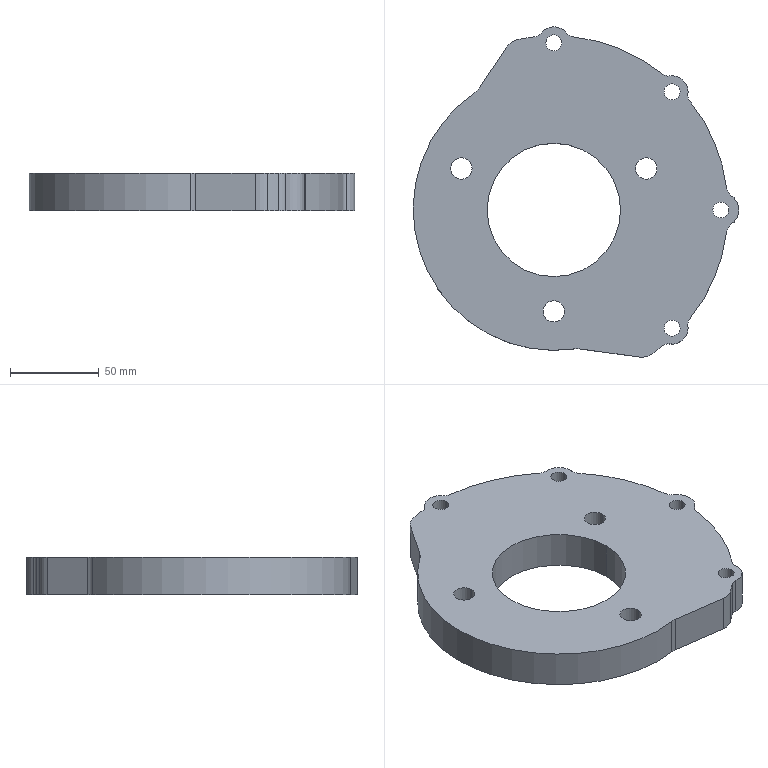Part | SolidWorks | features BaseBody 1 | 1 solid | 45 faces | box 183.112 x 185.815 x 21 mm | volume 422617 mm3 | cylinder 41 | plane 4 | commonest cylinder face diameters 9 x8 10 x8 12 x6 20 x6 18 x5 196 x5
STEP:
#1=CARTESIAN_POINT('',(4884.473,1068.014,21.));
#2=VERTEX_POINT('',#1);
#3=CARTESIAN_POINT('',(4894.755,1059.105,21.));
#4=VERTEX_POINT('',#3);
#5=CARTESIAN_POINT('',(4885.755,1059.105,21.));
#6=DIRECTION('',(0.,0.,-1.));
#7=DIRECTION('',(1.,0.,0.));
#8=AXIS2_PLACEMENT_3D('',#5,#6,#7);
#9=CIRCLE('',#8,9.);
#10=EDGE_CURVE('',#2,#4,#9,.T.);
#11=ORIENTED_EDGE('',*,*,#10,.T.);
#12=CARTESIAN_POINT('',(4894.755,1059.105,0.));
#13=VERTEX_POINT('',#12);
#14=CARTESIAN_POINT('',(4894.755,1059.105,21.));
#15=DIRECTION('',(0.,0.,-1.));
#16=VECTOR('',#15,1000.);
#17=LINE('',#14,#16);
#18=EDGE_CURVE('',#4,#13,#17,.T.);
#19=ORIENTED_EDGE('',*,*,#18,.T.);
#20=CARTESIAN_POINT('',(4884.473,1068.014,0.));
#21=VERTEX_POINT('',#20);
#22=CARTESIAN_POINT('',(4885.755,1059.105,0.));
#23=DIRECTION('',(0.,0.,-1.));
#24=DIRECTION('',(1.,0.,0.));
#25=AXIS2_PLACEMENT_3D('',#22,#23,#24);
#26=CIRCLE('',#25,9.);
#27=EDGE_CURVE('',#21,#13,#26,.T.);
#28=ORIENTED_EDGE('',*,*,#27,.F.);
#29=CARTESIAN_POINT('',(4884.473,1068.014,21.));
#30=DIRECTION('',(0.,0.,-1.));
#31=VECTOR('',#30,1000.);
#32=LINE('',#29,#31);
#33=EDGE_CURVE('',#2,#21,#32,.T.);
#34=ORIENTED_EDGE('',*,*,#33,.F.);
#35=EDGE_LOOP('',(#11,#19,#28,#34));
#36=FACE_OUTER_BOUND('',#35,.T.);
#37=CARTESIAN_POINT('',(4885.755,1059.105,21.));
#38=DIRECTION('',(0.,0.,-1.));
#39=DIRECTION('',(1.,0.,0.));
#40=AXIS2_PLACEMENT_3D('',#37,#38,#39);
#41=CYLINDRICAL_SURFACE('',#40,9.);
#42=ADVANCED_FACE('',(#36),#41,.T.);
#43=CARTESIAN_POINT('',(4918.777,1000.996,21.));
#44=VERTEX_POINT('',#43);
#45=CARTESIAN_POINT('',(4923.287,992.637,21.));
#46=VERTEX_POINT('',#45);
#47=CARTESIAN_POINT('',(4913.287,992.637,21.));
#48=DIRECTION('',(0.,0.,-1.));
#49=DIRECTION('',(1.,0.,0.));
#50=AXIS2_PLACEMENT_3D('',#47,#48,#49);
#51=CIRCLE('',#50,10.);
#52=EDGE_CURVE('',#44,#46,#51,.T.);
#53=ORIENTED_EDGE('',*,*,#52,.T.);
#54=CARTESIAN_POINT('',(4923.287,992.637,0.));
#55=VERTEX_POINT('',#54);
#56=CARTESIAN_POINT('',(4923.287,992.637,21.));
#57=DIRECTION('',(0.,0.,-1.));
#58=VECTOR('',#57,1000.);
#59=LINE('',#56,#58);
#60=EDGE_CURVE('',#46,#55,#59,.T.);
#61=ORIENTED_EDGE('',*,*,#60,.T.);
#62=CARTESIAN_POINT('',(4918.777,1000.996,0.));
#63=VERTEX_POINT('',#62);
#64=CARTESIAN_POINT('',(4913.287,992.637,0.));
#65=DIRECTION('',(0.,0.,-1.));
#66=DIRECTION('',(1.,0.,0.));
#67=AXIS2_PLACEMENT_3D('',#64,#65,#66);
#68=CIRCLE('',#67,10.);
#69=EDGE_CURVE('',#63,#55,#68,.T.);
#70=ORIENTED_EDGE('',*,*,#69,.F.);
#71=CARTESIAN_POINT('',(4918.777,1000.996,21.));
#72=DIRECTION('',(0.,0.,-1.));
#73=VECTOR('',#72,1000.);
#74=LINE('',#71,#73);
#75=EDGE_CURVE('',#44,#63,#74,.T.);
#76=ORIENTED_EDGE('',*,*,#75,.F.);
#77=EDGE_LOOP('',(#53,#61,#70,#76));
#78=FACE_OUTER_BOUND('',#77,.T.);
#79=CARTESIAN_POINT('',(4913.287,992.637,21.));
#80=DIRECTION('',(0.,0.,-1.));
#81=DIRECTION('',(1.,0.,0.));
#82=AXIS2_PLACEMENT_3D('',#79,#80,#81);
#83=CYLINDRICAL_SURFACE('',#82,10.);
#84=ADVANCED_FACE('',(#78),#83,.T.);
#85=CARTESIAN_POINT('',(4894.663,927.451,21.));
#86=VERTEX_POINT('',#85);
#87=CARTESIAN_POINT('',(4894.755,926.169,21.));
#88=VERTEX_POINT('',#87);
#89=CARTESIAN_POINT('',(4885.755,926.169,21.));
#90=DIRECTION('',(0.,0.,-1.));
#91=DIRECTION('',(1.,0.,0.));
#92=AXIS2_PLACEMENT_3D('',#89,#90,#91);
#93=CIRCLE('',#92,9.);
#94=EDGE_CURVE('',#86,#88,#93,.T.);
#95=ORIENTED_EDGE('',*,*,#94,.T.);
#96=CARTESIAN_POINT('',(4894.755,926.169,0.));
#97=VERTEX_POINT('',#96);
#98=CARTESIAN_POINT('',(4894.755,926.169,21.));
#99=DIRECTION('',(0.,0.,-1.));
#100=VECTOR('',#99,1000.);
#101=LINE('',#98,#100);
#102=EDGE_CURVE('',#88,#97,#101,.T.);
#103=ORIENTED_EDGE('',*,*,#102,.T.);
#104=CARTESIAN_POINT('',(4894.663,927.451,0.));
#105=VERTEX_POINT('',#104);
#106=CARTESIAN_POINT('',(4885.755,926.169,0.));
#107=DIRECTION('',(0.,0.,-1.));
#108=DIRECTION('',(1.,0.,0.));
#109=AXIS2_PLACEMENT_3D('',#106,#107,#108);
#110=CIRCLE('',#109,9.);
#111=EDGE_CURVE('',#105,#97,#110,.T.);
#112=ORIENTED_EDGE('',*,*,#111,.F.);
#113=CARTESIAN_POINT('',(4894.663,927.451,21.));
#114=DIRECTION('',(0.,0.,-1.));
#115=VECTOR('',#114,1000.);
#116=LINE('',#113,#115);
#117=EDGE_CURVE('',#86,#105,#116,.T.);
#118=ORIENTED_EDGE('',*,*,#117,.F.);
#119=EDGE_LOOP('',(#95,#103,#112,#118));
#120=FACE_OUTER_BOUND('',#119,.T.);
#121=CARTESIAN_POINT('',(4885.755,926.169,21.));
#122=DIRECTION('',(0.,0.,-1.));
#123=DIRECTION('',(1.,0.,0.));
#124=AXIS2_PLACEMENT_3D('',#121,#122,#123);
#125=CYLINDRICAL_SURFACE('',#124,9.);
#126=ADVANCED_FACE('',(#120),#125,.T.);
#127=CARTESIAN_POINT('',(4856.822,992.637,21.));
#128=VERTEX_POINT('',#127);
#129=CARTESIAN_POINT('',(4781.752,992.637,21.));
#130=VERTEX_POINT('',#129);
#131=CARTESIAN_POINT('',(4819.287,992.637,21.));
#132=DIRECTION('',(0.,0.,1.));
#133=DIRECTION('',(1.,0.,0.));
#134=AXIS2_PLACEMENT_3D('',#131,#132,#133);
#135=CIRCLE('',#134,37.535);
#136=EDGE_CURVE('',#128,#130,#135,.T.);
#137=ORIENTED_EDGE('',*,*,#136,.T.);
#138=CARTESIAN_POINT('',(4781.752,992.637,0.));
#139=VERTEX_POINT('',#138);
#140=CARTESIAN_POINT('',(4781.752,992.637,21.));
#141=DIRECTION('',(0.,0.,-1.));
#142=VECTOR('',#141,1000.);
#143=LINE('',#140,#142);
#144=EDGE_CURVE('',#130,#139,#143,.T.);
#145=ORIENTED_EDGE('',*,*,#144,.T.);
#146=CARTESIAN_POINT('',(4856.822,992.637,0.));
#147=VERTEX_POINT('',#146);
#148=CARTESIAN_POINT('',(4819.287,992.637,0.));
#149=DIRECTION('',(0.,0.,1.));
#150=DIRECTION('',(1.,0.,0.));
#151=AXIS2_PLACEMENT_3D('',#148,#149,#150);
#152=CIRCLE('',#151,37.535);
#153=EDGE_CURVE('',#147,#139,#152,.T.);
#154=ORIENTED_EDGE('',*,*,#153,.F.);
#155=CARTESIAN_POINT('',(4856.822,992.637,21.));
#156=DIRECTION('',(0.,0.,-1.));
#157=VECTOR('',#156,1000.);
#158=LINE('',#155,#157);
#159=EDGE_CURVE('',#128,#147,#158,.T.);
#160=ORIENTED_EDGE('',*,*,#159,.F.);
#161=EDGE_LOOP('',(#137,#145,#154,#160));
#162=FACE_OUTER_BOUND('',#161,.T.);
#163=CARTESIAN_POINT('',(4819.287,992.637,21.));
#164=DIRECTION('',(0.,0.,-1.));
#165=DIRECTION('',(1.,0.,0.));
#166=AXIS2_PLACEMENT_3D('',#163,#164,#165);
#167=CYLINDRICAL_SURFACE('',#166,37.535);
#168=ADVANCED_FACE('',(#162),#167,.F.);
#169=CARTESIAN_POINT('',(4825.287,935.637,21.));
#170=VERTEX_POINT('',#169);
#171=CARTESIAN_POINT('',(4813.287,935.637,21.));
#172=VERTEX_POINT('',#171);
#173=CARTESIAN_POINT('',(4819.287,935.637,21.));
#174=DIRECTION('',(0.,0.,1.));
#175=DIRECTION('',(1.,0.,0.));
#176=AXIS2_PLACEMENT_3D('',#173,#174,#175);
#177=CIRCLE('',#176,6.);
#178=EDGE_CURVE('',#170,#172,#177,.T.);
#179=ORIENTED_EDGE('',*,*,#178,.T.);
#180=CARTESIAN_POINT('',(4813.287,935.637,0.));
#181=VERTEX_POINT('',#180);
#182=CARTESIAN_POINT('',(4813.287,935.637,21.));
#183=DIRECTION('',(0.,0.,-1.));
#184=VECTOR('',#183,1000.);
#185=LINE('',#182,#184);
#186=EDGE_CURVE('',#172,#181,#185,.T.);
#187=ORIENTED_EDGE('',*,*,#186,.T.);
#188=CARTESIAN_POINT('',(4825.287,935.637,0.));
#189=VERTEX_POINT('',#188);
#190=CARTESIAN_POINT('',(4819.287,935.637,0.));
#191=DIRECTION('',(0.,0.,1.));
#192=DIRECTION('',(1.,0.,0.));
#193=AXIS2_PLACEMENT_3D('',#190,#191,#192);
#194=CIRCLE('',#193,6.);
#195=EDGE_CURVE('',#189,#181,#194,.T.);
#196=ORIENTED_EDGE('',*,*,#195,.F.);
#197=CARTESIAN_POINT('',(4825.287,935.637,21.));
#198=DIRECTION('',(0.,0.,-1.));
#199=VECTOR('',#198,1000.);
#200=LINE('',#197,#199);
#201=EDGE_CURVE('',#170,#189,#200,.T.);
#202=ORIENTED_EDGE('',*,*,#201,.F.);
#203=EDGE_LOOP('',(#179,#187,#196,#202));
#204=FACE_OUTER_BOUND('',#203,.T.);
#205=CARTESIAN_POINT('',(4819.287,935.637,21.));
#206=DIRECTION('',(0.,0.,-1.));
#207=DIRECTION('',(1.,0.,0.));
#208=AXIS2_PLACEMENT_3D('',#205,#206,#207);
#209=CYLINDRICAL_SURFACE('',#208,6.);
#210=ADVANCED_FACE('',(#204),#209,.F.);
#211=CARTESIAN_POINT('',(4823.787,1086.637,21.));
#212=VERTEX_POINT('',#211);
#213=CARTESIAN_POINT('',(4814.787,1086.637,21.));
#214=VERTEX_POINT('',#213);
#215=CARTESIAN_POINT('',(4819.287,1086.637,21.));
#216=DIRECTION('',(0.,0.,1.));
#217=DIRECTION('',(1.,0.,0.));
#218=AXIS2_PLACEMENT_3D('',#215,#216,#217);
#219=CIRCLE('',#218,4.5);
#220=EDGE_CURVE('',#212,#214,#219,.T.);
#221=ORIENTED_EDGE('',*,*,#220,.T.);
#222=CARTESIAN_POINT('',(4814.787,1086.637,0.));
#223=VERTEX_POINT('',#222);
#224=CARTESIAN_POINT('',(4814.787,1086.637,21.));
#225=DIRECTION('',(0.,0.,-1.));
#226=VECTOR('',#225,1000.);
#227=LINE('',#224,#226);
#228=EDGE_CURVE('',#214,#223,#227,.T.);
#229=ORIENTED_EDGE('',*,*,#228,.T.);
#230=CARTESIAN_POINT('',(4823.787,1086.637,0.));
#231=VERTEX_POINT('',#230);
#232=CARTESIAN_POINT('',(4819.287,1086.637,0.));
#233=DIRECTION('',(0.,0.,1.));
#234=DIRECTION('',(1.,0.,0.));
#235=AXIS2_PLACEMENT_3D('',#232,#233,#234);
#236=CIRCLE('',#235,4.5);
#237=EDGE_CURVE('',#231,#223,#236,.T.);
#238=ORIENTED_EDGE('',*,*,#237,.F.);
#239=CARTESIAN_POINT('',(4823.787,1086.637,21.));
#240=DIRECTION('',(0.,0.,-1.));
#241=VECTOR('',#240,1000.);
#242=LINE('',#239,#241);
#243=EDGE_CURVE('',#212,#231,#242,.T.);
#244=ORIENTED_EDGE('',*,*,#243,.F.);
#245=EDGE_LOOP('',(#221,#229,#238,#244));
#246=FACE_OUTER_BOUND('',#245,.T.);
#247=CARTESIAN_POINT('',(4819.287,1086.637,21.));
#248=DIRECTION('',(0.,0.,-1.));
#249=DIRECTION('',(1.,0.,0.));
#250=AXIS2_PLACEMENT_3D('',#247,#248,#249);
#251=CYLINDRICAL_SURFACE('',#250,4.5);
#252=ADVANCED_FACE('',(#246),#251,.F.);
#253=CARTESIAN_POINT('',(4877.287,1015.983,21.));
#254=VERTEX_POINT('',#253);
#255=CARTESIAN_POINT('',(4865.287,1015.983,21.));
#256=VERTEX_POINT('',#255);
#257=CARTESIAN_POINT('',(4871.287,1015.983,21.));
#258=DIRECTION('',(0.,0.,1.));
#259=DIRECTION('',(1.,0.,0.));
#260=AXIS2_PLACEMENT_3D('',#257,#258,#259);
#261=CIRCLE('',#260,6.);
#262=EDGE_CURVE('',#254,#256,#261,.T.);
#263=ORIENTED_EDGE('',*,*,#262,.T.);
#264=CARTESIAN_POINT('',(4865.287,1015.983,0.));
#265=VERTEX_POINT('',#264);
#266=CARTESIAN_POINT('',(4865.287,1015.983,21.));
#267=DIRECTION('',(0.,0.,-1.));
#268=VECTOR('',#267,1000.);
#269=LINE('',#266,#268);
#270=EDGE_CURVE('',#256,#265,#269,.T.);
#271=ORIENTED_EDGE('',*,*,#270,.T.);
#272=CARTESIAN_POINT('',(4877.287,1015.983,0.));
#273=VERTEX_POINT('',#272);
#274=CARTESIAN_POINT('',(4871.287,1015.983,0.));
#275=DIRECTION('',(0.,0.,1.));
#276=DIRECTION('',(1.,0.,0.));
#277=AXIS2_PLACEMENT_3D('',#274,#275,#276);
#278=CIRCLE('',#277,6.);
#279=EDGE_CURVE('',#273,#265,#278,.T.);
#280=ORIENTED_EDGE('',*,*,#279,.F.);
#281=CARTESIAN_POINT('',(4877.287,1015.983,21.));
#282=DIRECTION('',(0.,0.,-1.));
#283=VECTOR('',#282,1000.);
#284=LINE('',#281,#283);
#285=EDGE_CURVE('',#254,#273,#284,.T.);
#286=ORIENTED_EDGE('',*,*,#285,.F.);
#287=EDGE_LOOP('',(#263,#271,#280,#286));
#288=FACE_OUTER_BOUND('',#287,.T.);
#289=CARTESIAN_POINT('',(4871.287,1015.983,21.));
#290=DIRECTION('',(0.,0.,-1.));
#291=DIRECTION('',(1.,0.,0.));
#292=AXIS2_PLACEMENT_3D('',#289,#290,#291);
#293=CYLINDRICAL_SURFACE('',#292,6.);
#294=ADVANCED_FACE('',(#288),#293,.F.);
#295=CARTESIAN_POINT('',(4890.255,926.169,21.));
#296=VERTEX_POINT('',#295);
#297=CARTESIAN_POINT('',(4881.255,926.169,21.));
#298=VERTEX_POINT('',#297);
#299=CARTESIAN_POINT('',(4885.755,926.169,21.));
#300=DIRECTION('',(0.,0.,1.));
#301=DIRECTION('',(1.,0.,0.));
#302=AXIS2_PLACEMENT_3D('',#299,#300,#301);
#303=CIRCLE('',#302,4.5);
#304=EDGE_CURVE('',#296,#298,#303,.T.);
#305=ORIENTED_EDGE('',*,*,#304,.T.);
#306=CARTESIAN_POINT('',(4881.255,926.169,0.));
#307=VERTEX_POINT('',#306);
#308=CARTESIAN_POINT('',(4881.255,926.169,21.));
#309=DIRECTION('',(0.,0.,-1.));
#310=VECTOR('',#309,1000.);
#311=LINE('',#308,#310);
#312=EDGE_CURVE('',#298,#307,#311,.T.);
#313=ORIENTED_EDGE('',*,*,#312,.T.);
#314=CARTESIAN_POINT('',(4890.255,926.169,0.));
#315=VERTEX_POINT('',#314);
#316=CARTESIAN_POINT('',(4885.755,926.169,0.));
#317=DIRECTION('',(0.,0.,1.));
#318=DIRECTION('',(1.,0.,0.));
#319=AXIS2_PLACEMENT_3D('',#316,#317,#318);
#320=CIRCLE('',#319,4.5);
#321=EDGE_CURVE('',#315,#307,#320,.T.);
#322=ORIENTED_EDGE('',*,*,#321,.F.);
#323=CARTESIAN_POINT('',(4890.255,926.169,21.));
#324=DIRECTION('',(0.,0.,-1.));
#325=VECTOR('',#324,1000.);
#326=LINE('',#323,#325);
#327=EDGE_CURVE('',#296,#315,#326,.T.);
#328=ORIENTED_EDGE('',*,*,#327,.F.);
#329=EDGE_LOOP('',(#305,#313,#322,#328));
#330=FACE_OUTER_BOUND('',#329,.T.);
#331=CARTESIAN_POINT('',(4885.755,926.169,21.));
#332=DIRECTION('',(0.,0.,-1.));
#333=DIRECTION('',(1.,0.,0.));
#334=AXIS2_PLACEMENT_3D('',#331,#332,#333);
#335=CYLINDRICAL_SURFACE('',#334,4.5);
#336=ADVANCED_FACE('',(#330),#335,.F.);
#337=CARTESIAN_POINT('',(4890.255,1059.105,21.));
#338=VERTEX_POINT('',#337);
#339=CARTESIAN_POINT('',(4881.255,1059.105,21.));
#340=VERTEX_POINT('',#339);
#341=CARTESIAN_POINT('',(4885.755,1059.105,21.));
#342=DIRECTION('',(0.,0.,1.));
#343=DIRECTION('',(1.,0.,0.));
#344=AXIS2_PLACEMENT_3D('',#341,#342,#343);
#345=CIRCLE('',#344,4.5);
#346=EDGE_CURVE('',#338,#340,#345,.T.);
#347=ORIENTED_EDGE('',*,*,#346,.T.);
#348=CARTESIAN_POINT('',(4881.255,1059.105,0.));
#349=VERTEX_POINT('',#348);
#350=CARTESIAN_POINT('',(4881.255,1059.105,21.));
#351=DIRECTION('',(0.,0.,-1.));
#352=VECTOR('',#351,1000.);
#353=LINE('',#350,#352);
#354=EDGE_CURVE('',#340,#349,#353,.T.);
#355=ORIENTED_EDGE('',*,*,#354,.T.);
#356=CARTESIAN_POINT('',(4890.255,1059.105,0.));
#357=VERTEX_POINT('',#356);
#358=CARTESIAN_POINT('',(4885.755,1059.105,0.));
#359=DIRECTION('',(0.,0.,1.));
#360=DIRECTION('',(1.,0.,0.));
#361=AXIS2_PLACEMENT_3D('',#358,#359,#360);
#362=CIRCLE('',#361,4.5);
#363=EDGE_CURVE('',#357,#349,#362,.T.);
#364=ORIENTED_EDGE('',*,*,#363,.F.);
#365=CARTESIAN_POINT('',(4890.255,1059.105,21.));
#366=DIRECTION('',(0.,0.,-1.));
#367=VECTOR('',#366,1000.);
#368=LINE('',#365,#367);
#369=EDGE_CURVE('',#338,#357,#368,.T.);
#370=ORIENTED_EDGE('',*,*,#369,.F.);
#371=EDGE_LOOP('',(#347,#355,#364,#370));
#372=FACE_OUTER_BOUND('',#371,.T.);
#373=CARTESIAN_POINT('',(4885.755,1059.105,21.));
#374=DIRECTION('',(0.,0.,-1.));
#375=DIRECTION('',(1.,0.,0.));
#376=AXIS2_PLACEMENT_3D('',#373,#374,#375);
#377=CYLINDRICAL_SURFACE('',#376,4.5);
#378=ADVANCED_FACE('',(#372),#377,.F.);
#379=CARTESIAN_POINT('',(4917.787,992.637,21.));
#380=VERTEX_POINT('',#379);
#381=CARTESIAN_POINT('',(4908.787,992.637,21.));
#382=VERTEX_POINT('',#381);
#383=CARTESIAN_POINT('',(4913.287,992.637,21.));
#384=DIRECTION('',(0.,0.,1.));
#385=DIRECTION('',(1.,0.,0.));
#386=AXIS2_PLACEMENT_3D('',#383,#384,#385);
#387=CIRCLE('',#386,4.5);
#388=EDGE_CURVE('',#380,#382,#387,.T.);
#389=ORIENTED_EDGE('',*,*,#388,.T.);
#390=CARTESIAN_POINT('',(4908.787,992.637,0.));
#391=VERTEX_POINT('',#390);
#392=CARTESIAN_POINT('',(4908.787,992.637,21.));
#393=DIRECTION('',(0.,0.,-1.));
#394=VECTOR('',#393,1000.);
#395=LINE('',#392,#394);
#396=EDGE_CURVE('',#382,#391,#395,.T.);
#397=ORIENTED_EDGE('',*,*,#396,.T.);
#398=CARTESIAN_POINT('',(4917.787,992.637,0.));
#399=VERTEX_POINT('',#398);
#400=CARTESIAN_POINT('',(4913.287,992.637,0.));
#401=DIRECTION('',(0.,0.,1.));
#402=DIRECTION('',(1.,0.,0.));
#403=AXIS2_PLACEMENT_3D('',#400,#401,#402);
#404=CIRCLE('',#403,4.5);
#405=EDGE_CURVE('',#399,#391,#404,.T.);
#406=ORIENTED_EDGE('',*,*,#405,.F.);
#407=CARTESIAN_POINT('',(4917.787,992.637,21.));
#408=DIRECTION('',(0.,0.,-1.));
#409=VECTOR('',#408,1000.);
#410=LINE('',#407,#409);
#411=EDGE_CURVE('',#380,#399,#410,.T.);
#412=ORIENTED_EDGE('',*,*,#411,.F.);
#413=EDGE_LOOP('',(#389,#397,#406,#412));
#414=FACE_OUTER_BOUND('',#413,.T.);
#415=CARTESIAN_POINT('',(4913.287,992.637,21.));
#416=DIRECTION('',(0.,0.,-1.));
#417=DIRECTION('',(1.,0.,0.));
#418=AXIS2_PLACEMENT_3D('',#415,#416,#417);
#419=CYLINDRICAL_SURFACE('',#418,4.5);
#420=ADVANCED_FACE('',(#414),#419,.F.);
#421=CARTESIAN_POINT('',(4773.287,1015.983,21.));
#422=VERTEX_POINT('',#421);
#423=CARTESIAN_POINT('',(4761.287,1015.983,21.));
#424=VERTEX_POINT('',#423);
#425=CARTESIAN_POINT('',(4767.287,1015.983,21.));
#426=DIRECTION('',(0.,0.,1.));
#427=DIRECTION('',(1.,0.,0.));
#428=AXIS2_PLACEMENT_3D('',#425,#426,#427);
#429=CIRCLE('',#428,6.);
#430=EDGE_CURVE('',#422,#424,#429,.T.);
#431=ORIENTED_EDGE('',*,*,#430,.T.);
#432=CARTESIAN_POINT('',(4761.287,1015.983,0.));
#433=VERTEX_POINT('',#432);
#434=CARTESIAN_POINT('',(4761.287,1015.983,21.));
#435=DIRECTION('',(0.,0.,-1.));
#436=VECTOR('',#435,1000.);
#437=LINE('',#434,#436);
#438=EDGE_CURVE('',#424,#433,#437,.T.);
#439=ORIENTED_EDGE('',*,*,#438,.T.);
#440=CARTESIAN_POINT('',(4773.287,1015.983,0.));
#441=VERTEX_POINT('',#440);
#442=CARTESIAN_POINT('',(4767.287,1015.983,0.));
#443=DIRECTION('',(0.,0.,1.));
#444=DIRECTION('',(1.,0.,0.));
#445=AXIS2_PLACEMENT_3D('',#442,#443,#444);
#446=CIRCLE('',#445,6.);
#447=EDGE_CURVE('',#441,#433,#446,.T.);
#448=ORIENTED_EDGE('',*,*,#447,.F.);
#449=CARTESIAN_POINT('',(4773.287,1015.983,21.));
#450=DIRECTION('',(0.,0.,-1.));
#451=VECTOR('',#450,1000.);
#452=LINE('',#449,#451);
#453=EDGE_CURVE('',#422,#441,#452,.T.);
#454=ORIENTED_EDGE('',*,*,#453,.F.);
#455=EDGE_LOOP('',(#431,#439,#448,#454));
#456=FACE_OUTER_BOUND('',#455,.T.);
#457=CARTESIAN_POINT('',(4767.287,1015.983,21.));
#458=DIRECTION('',(0.,0.,-1.));
#459=DIRECTION('',(1.,0.,0.));
#460=AXIS2_PLACEMENT_3D('',#457,#458,#459);
#461=CYLINDRICAL_SURFACE('',#460,6.);
#462=ADVANCED_FACE('',(#456),#461,.F.);
#463=ORIENTED_EDGE('',*,*,#447,.T.);
#464=CARTESIAN_POINT('',(4767.287,1015.983,0.));
#465=DIRECTION('',(0.,0.,1.));
#466=DIRECTION('',(1.,0.,0.));
#467=AXIS2_PLACEMENT_3D('',#464,#465,#466);
#468=CIRCLE('',#467,6.);
#469=EDGE_CURVE('',#433,#441,#468,.T.);
#470=ORIENTED_EDGE('',*,*,#469,.T.);
#471=EDGE_LOOP('',(#463,#470));
#472=FACE_BOUND('',#471,.T.);
#473=ORIENTED_EDGE('',*,*,#153,.T.);
#474=CARTESIAN_POINT('',(4819.287,992.637,0.));
#475=DIRECTION('',(0.,0.,1.));
#476=DIRECTION('',(1.,0.,0.));
#477=AXIS2_PLACEMENT_3D('',#474,#475,#476);
#478=CIRCLE('',#477,37.535);
#479=EDGE_CURVE('',#139,#147,#478,.T.);
#480=ORIENTED_EDGE('',*,*,#479,.T.);
#481=EDGE_LOOP('',(#473,#480));
#482=FACE_BOUND('',#481,.T.);
#483=ORIENTED_EDGE('',*,*,#195,.T.);
#484=CARTESIAN_POINT('',(4819.287,935.637,0.));
#485=DIRECTION('',(0.,0.,1.));
#486=DIRECTION('',(1.,0.,0.));
#487=AXIS2_PLACEMENT_3D('',#484,#485,#486);
#488=CIRCLE('',#487,6.);
#489=EDGE_CURVE('',#181,#189,#488,.T.);
#490=ORIENTED_EDGE('',*,*,#489,.T.);
#491=EDGE_LOOP('',(#483,#490));
#492=FACE_BOUND('',#491,.T.);
#493=ORIENTED_EDGE('',*,*,#237,.T.);
#494=CARTESIAN_POINT('',(4819.287,1086.637,0.));
#495=DIRECTION('',(0.,0.,1.));
#496=DIRECTION('',(1.,0.,0.));
#497=AXIS2_PLACEMENT_3D('',#494,#495,#496);
#498=CIRCLE('',#497,4.5);
#499=EDGE_CURVE('',#223,#231,#498,.T.);
#500=ORIENTED_EDGE('',*,*,#499,.T.);
#501=EDGE_LOOP('',(#493,#500));
#502=FACE_BOUND('',#501,.T.);
#503=ORIENTED_EDGE('',*,*,#279,.T.);
#504=CARTESIAN_POINT('',(4871.287,1015.983,0.));
#505=DIRECTION('',(0.,0.,1.));
#506=DIRECTION('',(1.,0.,0.));
#507=AXIS2_PLACEMENT_3D('',#504,#505,#506);
#508=CIRCLE('',#507,6.);
#509=EDGE_CURVE('',#265,#273,#508,.T.);
#510=ORIENTED_EDGE('',*,*,#509,.T.);
#511=EDGE_LOOP('',(#503,#510));
#512=FACE_BOUND('',#511,.T.);
#513=ORIENTED_EDGE('',*,*,#321,.T.);
#514=CARTESIAN_POINT('',(4885.755,926.169,0.));
#515=DIRECTION('',(0.,0.,1.));
#516=DIRECTION('',(1.,0.,0.));
#517=AXIS2_PLACEMENT_3D('',#514,#515,#516);
#518=CIRCLE('',#517,4.5);
#519=EDGE_CURVE('',#307,#315,#518,.T.);
#520=ORIENTED_EDGE('',*,*,#519,.T.);
#521=EDGE_LOOP('',(#513,#520));
#522=FACE_BOUND('',#521,.T.);
#523=ORIENTED_EDGE('',*,*,#363,.T.);
#524=CARTESIAN_POINT('',(4885.755,1059.105,0.));
#525=DIRECTION('',(0.,0.,1.));
#526=DIRECTION('',(1.,0.,0.));
#527=AXIS2_PLACEMENT_3D('',#524,#525,#526);
#528=CIRCLE('',#527,4.5);
#529=EDGE_CURVE('',#349,#357,#528,.T.);
#530=ORIENTED_EDGE('',*,*,#529,.T.);
#531=EDGE_LOOP('',(#523,#530));
#532=FACE_BOUND('',#531,.T.);
#533=ORIENTED_EDGE('',*,*,#405,.T.);
#534=CARTESIAN_POINT('',(4913.287,992.637,0.));
#535=DIRECTION('',(0.,0.,1.));
#536=DIRECTION('',(1.,0.,0.));
#537=AXIS2_PLACEMENT_3D('',#534,#535,#536);
#538=CIRCLE('',#537,4.5);
#539=EDGE_CURVE('',#391,#399,#538,.T.);
#540=ORIENTED_EDGE('',*,*,#539,.T.);
#541=EDGE_LOOP('',(#533,#540));
#542=FACE_BOUND('',#541,.T.);
#543=CARTESIAN_POINT('',(4830.945,914.487,0.));
#544=VERTEX_POINT('',#543);
#545=CARTESIAN_POINT('',(4774.725,1058.565,0.));
#546=VERTEX_POINT('',#545);
#547=CARTESIAN_POINT('',(4819.561,993.052,0.));
#548=DIRECTION('',(0.,0.,-1.));
#549=DIRECTION('',(1.,0.,0.));
#550=AXIS2_PLACEMENT_3D('',#547,#548,#549);
#551=CIRCLE('',#550,79.386);
#552=EDGE_CURVE('',#544,#546,#551,.T.);
#553=ORIENTED_EDGE('',*,*,#552,.T.);
#554=CARTESIAN_POINT('',(4777.398,1061.27,0.));
#555=VERTEX_POINT('',#554);
#556=CARTESIAN_POINT('',(4769.077,1066.817,0.));
#557=DIRECTION('',(0.,0.,1.));
#558=DIRECTION('',(1.,0.,0.));
#559=AXIS2_PLACEMENT_3D('',#556,#557,#558);
#560=CIRCLE('',#559,10.);
#561=EDGE_CURVE('',#546,#555,#560,.T.);
#562=ORIENTED_EDGE('',*,*,#561,.T.);
#563=CARTESIAN_POINT('',(4792.734,1084.275,0.));
#564=VERTEX_POINT('',#563);
#565=CARTESIAN_POINT('',(4777.398,1061.27,0.));
#566=DIRECTION('',(0.5547,0.8321,0.));
#567=VECTOR('',#566,1000.);
#568=LINE('',#565,#567);
#569=EDGE_CURVE('',#555,#564,#568,.T.);
#570=ORIENTED_EDGE('',*,*,#569,.T.);
#571=CARTESIAN_POINT('',(4798.983,1088.511,0.));
#572=VERTEX_POINT('',#571);
#573=CARTESIAN_POINT('',(4801.055,1078.728,0.));
#574=DIRECTION('',(0.,0.,-1.));
#575=DIRECTION('',(1.,0.,0.));
#576=AXIS2_PLACEMENT_3D('',#573,#574,#575);
#577=CIRCLE('',#576,10.);
#578=EDGE_CURVE('',#564,#572,#577,.T.);
#579=ORIENTED_EDGE('',*,*,#578,.T.);
#580=CARTESIAN_POINT('',(4808.622,1090.055,0.));
#581=VERTEX_POINT('',#580);
#582=CARTESIAN_POINT('',(4819.287,992.637,0.));
#583=DIRECTION('',(0.,0.,-1.));
#584=DIRECTION('',(1.,0.,0.));
#585=AXIS2_PLACEMENT_3D('',#582,#583,#584);
#586=CIRCLE('',#585,98.);
#587=EDGE_CURVE('',#572,#581,#586,.T.);
#588=ORIENTED_EDGE('',*,*,#587,.T.);
#589=CARTESIAN_POINT('',(4812.082,1092.03,0.));
#590=VERTEX_POINT('',#589);
#591=CARTESIAN_POINT('',(4808.078,1095.026,0.));
#592=DIRECTION('',(0.,0.,1.));
#593=DIRECTION('',(1.,0.,0.));
#594=AXIS2_PLACEMENT_3D('',#591,#592,#593);
#595=CIRCLE('',#594,5.);
#596=EDGE_CURVE('',#581,#590,#595,.T.);
#597=ORIENTED_EDGE('',*,*,#596,.T.);
#598=CARTESIAN_POINT('',(4826.493,1092.03,0.));
#599=VERTEX_POINT('',#598);
#600=CARTESIAN_POINT('',(4819.287,1086.637,0.));
#601=DIRECTION('',(0.,0.,-1.));
#602=DIRECTION('',(1.,0.,0.));
#603=AXIS2_PLACEMENT_3D('',#600,#601,#602);
#604=CIRCLE('',#603,9.);
#605=EDGE_CURVE('',#590,#599,#604,.T.);
#606=ORIENTED_EDGE('',*,*,#605,.T.);
#607=CARTESIAN_POINT('',(4829.952,1090.055,0.));
#608=VERTEX_POINT('',#607);
#609=CARTESIAN_POINT('',(4830.496,1095.026,0.));
#610=DIRECTION('',(0.,0.,1.));
#611=DIRECTION('',(1.,0.,0.));
#612=AXIS2_PLACEMENT_3D('',#609,#610,#611);
#613=CIRCLE('',#612,5.);
#614=EDGE_CURVE('',#599,#608,#613,.T.);
#615=ORIENTED_EDGE('',*,*,#614,.T.);
#616=CARTESIAN_POINT('',(4880.631,1069.063,0.));
#617=VERTEX_POINT('',#616);
#618=CARTESIAN_POINT('',(4819.287,992.637,0.));
#619=DIRECTION('',(0.,0.,-1.));
#620=DIRECTION('',(1.,0.,0.));
#621=AXIS2_PLACEMENT_3D('',#618,#619,#620);
#622=CIRCLE('',#621,98.);
#623=EDGE_CURVE('',#608,#617,#622,.T.);
#624=ORIENTED_EDGE('',*,*,#623,.T.);
#625=CARTESIAN_POINT('',(4883.761,1072.963,0.));
#626=DIRECTION('',(0.,0.,1.));
#627=DIRECTION('',(1.,0.,0.));
#628=AXIS2_PLACEMENT_3D('',#625,#626,#627);
#629=CIRCLE('',#628,5.);
#630=EDGE_CURVE('',#617,#21,#629,.T.);
#631=ORIENTED_EDGE('',*,*,#630,.T.);
#632=ORIENTED_EDGE('',*,*,#27,.T.);
#633=CARTESIAN_POINT('',(4894.663,1057.823,0.));
#634=VERTEX_POINT('',#633);
#635=CARTESIAN_POINT('',(4885.755,1059.105,0.));
#636=DIRECTION('',(0.,0.,-1.));
#637=DIRECTION('',(1.,0.,0.));
#638=AXIS2_PLACEMENT_3D('',#635,#636,#637);
#639=CIRCLE('',#638,9.);
#640=EDGE_CURVE('',#13,#634,#639,.T.);
#641=ORIENTED_EDGE('',*,*,#640,.T.);
#642=CARTESIAN_POINT('',(4895.713,1053.981,0.));
#643=VERTEX_POINT('',#642);
#644=CARTESIAN_POINT('',(4899.612,1057.111,0.));
#645=DIRECTION('',(0.,0.,1.));
#646=DIRECTION('',(1.,0.,0.));
#647=AXIS2_PLACEMENT_3D('',#644,#645,#646);
#648=CIRCLE('',#647,5.);
#649=EDGE_CURVE('',#634,#643,#648,.T.);
#650=ORIENTED_EDGE('',*,*,#649,.T.);
#651=CARTESIAN_POINT('',(4916.558,1004.567,0.));
#652=VERTEX_POINT('',#651);
#653=CARTESIAN_POINT('',(4819.287,992.637,0.));
#654=DIRECTION('',(0.,0.,-1.));
#655=DIRECTION('',(1.,0.,0.));
#656=AXIS2_PLACEMENT_3D('',#653,#654,#655);
#657=CIRCLE('',#656,98.);
#658=EDGE_CURVE('',#643,#652,#657,.T.);
#659=ORIENTED_EDGE('',*,*,#658,.T.);
#660=CARTESIAN_POINT('',(4921.521,1005.175,0.));
#661=DIRECTION('',(0.,0.,1.));
#662=DIRECTION('',(1.,0.,0.));
#663=AXIS2_PLACEMENT_3D('',#660,#661,#662);
#664=CIRCLE('',#663,5.);
#665=EDGE_CURVE('',#652,#63,#664,.T.);
#666=ORIENTED_EDGE('',*,*,#665,.T.);
#667=ORIENTED_EDGE('',*,*,#69,.T.);
#668=CARTESIAN_POINT('',(4918.777,984.279,0.));
#669=VERTEX_POINT('',#668);
#670=CARTESIAN_POINT('',(4913.287,992.637,0.));
#671=DIRECTION('',(0.,0.,-1.));
#672=DIRECTION('',(1.,0.,0.));
#673=AXIS2_PLACEMENT_3D('',#670,#671,#672);
#674=CIRCLE('',#673,10.);
#675=EDGE_CURVE('',#55,#669,#674,.T.);
#676=ORIENTED_EDGE('',*,*,#675,.T.);
#677=CARTESIAN_POINT('',(4916.558,980.708,0.));
#678=VERTEX_POINT('',#677);
#679=CARTESIAN_POINT('',(4921.521,980.099,0.));
#680=DIRECTION('',(0.,0.,1.));
#681=DIRECTION('',(1.,0.,0.));
#682=AXIS2_PLACEMENT_3D('',#679,#680,#681);
#683=CIRCLE('',#682,5.);
#684=EDGE_CURVE('',#669,#678,#683,.T.);
#685=ORIENTED_EDGE('',*,*,#684,.T.);
#686=CARTESIAN_POINT('',(4895.713,931.293,0.));
#687=VERTEX_POINT('',#686);
#688=CARTESIAN_POINT('',(4819.287,992.637,0.));
#689=DIRECTION('',(0.,0.,-1.));
#690=DIRECTION('',(1.,0.,0.));
#691=AXIS2_PLACEMENT_3D('',#688,#689,#690);
#692=CIRCLE('',#691,98.);
#693=EDGE_CURVE('',#678,#687,#692,.T.);
#694=ORIENTED_EDGE('',*,*,#693,.T.);
#695=CARTESIAN_POINT('',(4899.612,928.164,0.));
#696=DIRECTION('',(0.,0.,1.));
#697=DIRECTION('',(1.,0.,0.));
#698=AXIS2_PLACEMENT_3D('',#695,#696,#697);
#699=CIRCLE('',#698,5.);
#700=EDGE_CURVE('',#687,#105,#699,.T.);
#701=ORIENTED_EDGE('',*,*,#700,.T.);
#702=ORIENTED_EDGE('',*,*,#111,.T.);
#703=CARTESIAN_POINT('',(4884.473,917.261,0.));
#704=VERTEX_POINT('',#703);
#705=CARTESIAN_POINT('',(4885.755,926.169,0.));
#706=DIRECTION('',(0.,0.,-1.));
#707=DIRECTION('',(1.,0.,0.));
#708=AXIS2_PLACEMENT_3D('',#705,#706,#707);
#709=CIRCLE('',#708,9.);
#710=EDGE_CURVE('',#97,#704,#709,.T.);
#711=ORIENTED_EDGE('',*,*,#710,.T.);
#712=CARTESIAN_POINT('',(4880.631,916.211,0.));
#713=VERTEX_POINT('',#712);
#714=CARTESIAN_POINT('',(4883.761,912.312,0.));
#715=DIRECTION('',(0.,0.,1.));
#716=DIRECTION('',(1.,0.,0.));
#717=AXIS2_PLACEMENT_3D('',#714,#715,#716);
#718=CIRCLE('',#717,5.);
#719=EDGE_CURVE('',#704,#713,#718,.T.);
#720=ORIENTED_EDGE('',*,*,#719,.T.);
#721=CARTESIAN_POINT('',(4874.318,911.547,0.));
#722=VERTEX_POINT('',#721);
#723=CARTESIAN_POINT('',(4819.287,992.637,0.));
#724=DIRECTION('',(0.,0.,-1.));
#725=DIRECTION('',(1.,0.,0.));
#726=AXIS2_PLACEMENT_3D('',#723,#724,#725);
#727=CIRCLE('',#726,98.);
#728=EDGE_CURVE('',#713,#722,#727,.T.);
#729=ORIENTED_EDGE('',*,*,#728,.T.);
#730=CARTESIAN_POINT('',(4867.352,909.914,0.));
#731=VERTEX_POINT('',#730);
#732=CARTESIAN_POINT('',(4868.703,919.822,0.));
#733=DIRECTION('',(0.,0.,-1.));
#734=DIRECTION('',(1.,0.,0.));
#735=AXIS2_PLACEMENT_3D('',#732,#733,#734);
#736=CIRCLE('',#735,10.);
#737=EDGE_CURVE('',#722,#731,#736,.T.);
#738=ORIENTED_EDGE('',*,*,#737,.T.);
#739=CARTESIAN_POINT('',(4833.73,914.498,0.));
#740=VERTEX_POINT('',#739);
#741=CARTESIAN_POINT('',(4867.352,909.914,0.));
#742=DIRECTION('',(-0.9908,0.1351,0.));
#743=VECTOR('',#742,1000.);
#744=LINE('',#741,#743);
#745=EDGE_CURVE('',#731,#740,#744,.T.);
#746=ORIENTED_EDGE('',*,*,#745,.T.);
#747=CARTESIAN_POINT('',(4832.379,904.59,0.));
#748=DIRECTION('',(0.,0.,1.));
#749=DIRECTION('',(1.,0.,0.));
#750=AXIS2_PLACEMENT_3D('',#747,#748,#749);
#751=CIRCLE('',#750,10.);
#752=EDGE_CURVE('',#740,#544,#751,.T.);
#753=ORIENTED_EDGE('',*,*,#752,.T.);
#754=EDGE_LOOP('',(#553,#562,#570,#579,#588,#597,#606,#615,#624,#631,#632,#641,#650,#659,#666,#667,#676,#685,#694,#701,#702,#711,#720,#729,#738,#746,#753));
#755=FACE_OUTER_BOUND('',#754,.T.);
#756=CARTESIAN_POINT('',(4819.561,993.052,0.));
#757=DIRECTION('',(0.,0.,-1.));
#758=DIRECTION('',(0.,-1.,0.));
#759=AXIS2_PLACEMENT_3D('',#756,#757,#758);
#760=PLANE('',#759);
#761=ADVANCED_FACE('',(#472,#482,#492,#502,#512,#522,#532,#542,#755),#760,.T.);
#762=ORIENTED_EDGE('',*,*,#430,.F.);
#763=CARTESIAN_POINT('',(4767.287,1015.983,21.));
#764=DIRECTION('',(0.,0.,1.));
#765=DIRECTION('',(1.,0.,0.));
#766=AXIS2_PLACEMENT_3D('',#763,#764,#765);
#767=CIRCLE('',#766,6.);
#768=EDGE_CURVE('',#424,#422,#767,.T.);
#769=ORIENTED_EDGE('',*,*,#768,.F.);
#770=EDGE_LOOP('',(#762,#769));
#771=FACE_BOUND('',#770,.T.);
#772=ORIENTED_EDGE('',*,*,#136,.F.);
#773=CARTESIAN_POINT('',(4819.287,992.637,21.));
#774=DIRECTION('',(0.,0.,1.));
#775=DIRECTION('',(1.,0.,0.));
#776=AXIS2_PLACEMENT_3D('',#773,#774,#775);
#777=CIRCLE('',#776,37.535);
#778=EDGE_CURVE('',#130,#128,#777,.T.);
#779=ORIENTED_EDGE('',*,*,#778,.F.);
#780=EDGE_LOOP('',(#772,#779));
#781=FACE_BOUND('',#780,.T.);
#782=ORIENTED_EDGE('',*,*,#178,.F.);
#783=CARTESIAN_POINT('',(4819.287,935.637,21.));
#784=DIRECTION('',(0.,0.,1.));
#785=DIRECTION('',(1.,0.,0.));
#786=AXIS2_PLACEMENT_3D('',#783,#784,#785);
#787=CIRCLE('',#786,6.);
#788=EDGE_CURVE('',#172,#170,#787,.T.);
#789=ORIENTED_EDGE('',*,*,#788,.F.);
#790=EDGE_LOOP('',(#782,#789));
#791=FACE_BOUND('',#790,.T.);
#792=ORIENTED_EDGE('',*,*,#220,.F.);
#793=CARTESIAN_POINT('',(4819.287,1086.637,21.));
#794=DIRECTION('',(0.,0.,1.));
#795=DIRECTION('',(1.,0.,0.));
#796=AXIS2_PLACEMENT_3D('',#793,#794,#795);
#797=CIRCLE('',#796,4.5);
#798=EDGE_CURVE('',#214,#212,#797,.T.);
#799=ORIENTED_EDGE('',*,*,#798,.F.);
#800=EDGE_LOOP('',(#792,#799));
#801=FACE_BOUND('',#800,.T.);
#802=ORIENTED_EDGE('',*,*,#262,.F.);
#803=CARTESIAN_POINT('',(4871.287,1015.983,21.));
#804=DIRECTION('',(0.,0.,1.));
#805=DIRECTION('',(1.,0.,0.));
#806=AXIS2_PLACEMENT_3D('',#803,#804,#805);
#807=CIRCLE('',#806,6.);
#808=EDGE_CURVE('',#256,#254,#807,.T.);
#809=ORIENTED_EDGE('',*,*,#808,.F.);
#810=EDGE_LOOP('',(#802,#809));
#811=FACE_BOUND('',#810,.T.);
#812=ORIENTED_EDGE('',*,*,#304,.F.);
#813=CARTESIAN_POINT('',(4885.755,926.169,21.));
#814=DIRECTION('',(0.,0.,1.));
#815=DIRECTION('',(1.,0.,0.));
#816=AXIS2_PLACEMENT_3D('',#813,#814,#815);
#817=CIRCLE('',#816,4.5);
#818=EDGE_CURVE('',#298,#296,#817,.T.);
#819=ORIENTED_EDGE('',*,*,#818,.F.);
#820=EDGE_LOOP('',(#812,#819));
#821=FACE_BOUND('',#820,.T.);
#822=ORIENTED_EDGE('',*,*,#346,.F.);
#823=CARTESIAN_POINT('',(4885.755,1059.105,21.));
#824=DIRECTION('',(0.,0.,1.));
#825=DIRECTION('',(1.,0.,0.));
#826=AXIS2_PLACEMENT_3D('',#823,#824,#825);
#827=CIRCLE('',#826,4.5);
#828=EDGE_CURVE('',#340,#338,#827,.T.);
#829=ORIENTED_EDGE('',*,*,#828,.F.);
#830=EDGE_LOOP('',(#822,#829));
#831=FACE_BOUND('',#830,.T.);
#832=ORIENTED_EDGE('',*,*,#388,.F.);
#833=CARTESIAN_POINT('',(4913.287,992.637,21.));
#834=DIRECTION('',(0.,0.,1.));
#835=DIRECTION('',(1.,0.,0.));
#836=AXIS2_PLACEMENT_3D('',#833,#834,#835);
#837=CIRCLE('',#836,4.5);
#838=EDGE_CURVE('',#382,#380,#837,.T.);
#839=ORIENTED_EDGE('',*,*,#838,.F.);
#840=EDGE_LOOP('',(#832,#839));
#841=FACE_BOUND('',#840,.T.);
#842=CARTESIAN_POINT('',(4830.945,914.487,21.));
#843=VERTEX_POINT('',#842);
#844=CARTESIAN_POINT('',(4774.725,1058.565,21.));
#845=VERTEX_POINT('',#844);
#846=CARTESIAN_POINT('',(4819.561,993.052,21.));
#847=DIRECTION('',(0.,0.,-1.));
#848=DIRECTION('',(1.,0.,0.));
#849=AXIS2_PLACEMENT_3D('',#846,#847,#848);
#850=CIRCLE('',#849,79.386);
#851=EDGE_CURVE('',#843,#845,#850,.T.);
#852=ORIENTED_EDGE('',*,*,#851,.F.);
#853=CARTESIAN_POINT('',(4833.73,914.498,21.));
#854=VERTEX_POINT('',#853);
#855=CARTESIAN_POINT('',(4832.379,904.59,21.));
#856=DIRECTION('',(0.,0.,1.));
#857=DIRECTION('',(1.,0.,0.));
#858=AXIS2_PLACEMENT_3D('',#855,#856,#857);
#859=CIRCLE('',#858,10.);
#860=EDGE_CURVE('',#854,#843,#859,.T.);
#861=ORIENTED_EDGE('',*,*,#860,.F.);
#862=CARTESIAN_POINT('',(4867.352,909.914,21.));
#863=VERTEX_POINT('',#862);
#864=CARTESIAN_POINT('',(4867.352,909.914,21.));
#865=DIRECTION('',(-0.9908,0.1351,0.));
#866=VECTOR('',#865,1000.);
#867=LINE('',#864,#866);
#868=EDGE_CURVE('',#863,#854,#867,.T.);
#869=ORIENTED_EDGE('',*,*,#868,.F.);
#870=CARTESIAN_POINT('',(4874.318,911.547,21.));
#871=VERTEX_POINT('',#870);
#872=CARTESIAN_POINT('',(4868.703,919.822,21.));
#873=DIRECTION('',(0.,0.,-1.));
#874=DIRECTION('',(1.,0.,0.));
#875=AXIS2_PLACEMENT_3D('',#872,#873,#874);
#876=CIRCLE('',#875,10.);
#877=EDGE_CURVE('',#871,#863,#876,.T.);
#878=ORIENTED_EDGE('',*,*,#877,.F.);
#879=CARTESIAN_POINT('',(4880.631,916.211,21.));
#880=VERTEX_POINT('',#879);
#881=CARTESIAN_POINT('',(4819.287,992.637,21.));
#882=DIRECTION('',(0.,0.,-1.));
#883=DIRECTION('',(1.,0.,0.));
#884=AXIS2_PLACEMENT_3D('',#881,#882,#883);
#885=CIRCLE('',#884,98.);
#886=EDGE_CURVE('',#880,#871,#885,.T.);
#887=ORIENTED_EDGE('',*,*,#886,.F.);
#888=CARTESIAN_POINT('',(4884.473,917.261,21.));
#889=VERTEX_POINT('',#888);
#890=CARTESIAN_POINT('',(4883.761,912.312,21.));
#891=DIRECTION('',(0.,0.,1.));
#892=DIRECTION('',(1.,0.,0.));
#893=AXIS2_PLACEMENT_3D('',#890,#891,#892);
#894=CIRCLE('',#893,5.);
#895=EDGE_CURVE('',#889,#880,#894,.T.);
#896=ORIENTED_EDGE('',*,*,#895,.F.);
#897=CARTESIAN_POINT('',(4885.755,926.169,21.));
#898=DIRECTION('',(0.,0.,-1.));
#899=DIRECTION('',(1.,0.,0.));
#900=AXIS2_PLACEMENT_3D('',#897,#898,#899);
#901=CIRCLE('',#900,9.);
#902=EDGE_CURVE('',#88,#889,#901,.T.);
#903=ORIENTED_EDGE('',*,*,#902,.F.);
#904=ORIENTED_EDGE('',*,*,#94,.F.);
#905=CARTESIAN_POINT('',(4895.713,931.293,21.));
#906=VERTEX_POINT('',#905);
#907=CARTESIAN_POINT('',(4899.612,928.164,21.));
#908=DIRECTION('',(0.,0.,1.));
#909=DIRECTION('',(1.,0.,0.));
#910=AXIS2_PLACEMENT_3D('',#907,#908,#909);
#911=CIRCLE('',#910,5.);
#912=EDGE_CURVE('',#906,#86,#911,.T.);
#913=ORIENTED_EDGE('',*,*,#912,.F.);
#914=CARTESIAN_POINT('',(4916.558,980.708,21.));
#915=VERTEX_POINT('',#914);
#916=CARTESIAN_POINT('',(4819.287,992.637,21.));
#917=DIRECTION('',(0.,0.,-1.));
#918=DIRECTION('',(1.,0.,0.));
#919=AXIS2_PLACEMENT_3D('',#916,#917,#918);
#920=CIRCLE('',#919,98.);
#921=EDGE_CURVE('',#915,#906,#920,.T.);
#922=ORIENTED_EDGE('',*,*,#921,.F.);
#923=CARTESIAN_POINT('',(4918.777,984.279,21.));
#924=VERTEX_POINT('',#923);
#925=CARTESIAN_POINT('',(4921.521,980.099,21.));
#926=DIRECTION('',(0.,0.,1.));
#927=DIRECTION('',(1.,0.,0.));
#928=AXIS2_PLACEMENT_3D('',#925,#926,#927);
#929=CIRCLE('',#928,5.);
#930=EDGE_CURVE('',#924,#915,#929,.T.);
#931=ORIENTED_EDGE('',*,*,#930,.F.);
#932=CARTESIAN_POINT('',(4913.287,992.637,21.));
#933=DIRECTION('',(0.,0.,-1.));
#934=DIRECTION('',(1.,0.,0.));
#935=AXIS2_PLACEMENT_3D('',#932,#933,#934);
#936=CIRCLE('',#935,10.);
#937=EDGE_CURVE('',#46,#924,#936,.T.);
#938=ORIENTED_EDGE('',*,*,#937,.F.);
#939=ORIENTED_EDGE('',*,*,#52,.F.);
#940=CARTESIAN_POINT('',(4916.558,1004.567,21.));
#941=VERTEX_POINT('',#940);
#942=CARTESIAN_POINT('',(4921.521,1005.175,21.));
#943=DIRECTION('',(0.,0.,1.));
#944=DIRECTION('',(1.,0.,0.));
#945=AXIS2_PLACEMENT_3D('',#942,#943,#944);
#946=CIRCLE('',#945,5.);
#947=EDGE_CURVE('',#941,#44,#946,.T.);
#948=ORIENTED_EDGE('',*,*,#947,.F.);
#949=CARTESIAN_POINT('',(4895.713,1053.981,21.));
#950=VERTEX_POINT('',#949);
#951=CARTESIAN_POINT('',(4819.287,992.637,21.));
#952=DIRECTION('',(0.,0.,-1.));
#953=DIRECTION('',(1.,0.,0.));
#954=AXIS2_PLACEMENT_3D('',#951,#952,#953);
#955=CIRCLE('',#954,98.);
#956=EDGE_CURVE('',#950,#941,#955,.T.);
#957=ORIENTED_EDGE('',*,*,#956,.F.);
#958=CARTESIAN_POINT('',(4894.663,1057.823,21.));
#959=VERTEX_POINT('',#958);
#960=CARTESIAN_POINT('',(4899.612,1057.111,21.));
#961=DIRECTION('',(0.,0.,1.));
#962=DIRECTION('',(1.,0.,0.));
#963=AXIS2_PLACEMENT_3D('',#960,#961,#962);
#964=CIRCLE('',#963,5.);
#965=EDGE_CURVE('',#959,#950,#964,.T.);
#966=ORIENTED_EDGE('',*,*,#965,.F.);
#967=CARTESIAN_POINT('',(4885.755,1059.105,21.));
#968=DIRECTION('',(0.,0.,-1.));
#969=DIRECTION('',(1.,0.,0.));
#970=AXIS2_PLACEMENT_3D('',#967,#968,#969);
#971=CIRCLE('',#970,9.);
#972=EDGE_CURVE('',#4,#959,#971,.T.);
#973=ORIENTED_EDGE('',*,*,#972,.F.);
#974=ORIENTED_EDGE('',*,*,#10,.F.);
#975=CARTESIAN_POINT('',(4880.631,1069.063,21.));
#976=VERTEX_POINT('',#975);
#977=CARTESIAN_POINT('',(4883.761,1072.963,21.));
#978=DIRECTION('',(0.,0.,1.));
#979=DIRECTION('',(1.,0.,0.));
#980=AXIS2_PLACEMENT_3D('',#977,#978,#979);
#981=CIRCLE('',#980,5.);
#982=EDGE_CURVE('',#976,#2,#981,.T.);
#983=ORIENTED_EDGE('',*,*,#982,.F.);
#984=CARTESIAN_POINT('',(4829.952,1090.055,21.));
#985=VERTEX_POINT('',#984);
#986=CARTESIAN_POINT('',(4819.287,992.637,21.));
#987=DIRECTION('',(0.,0.,-1.));
#988=DIRECTION('',(1.,0.,0.));
#989=AXIS2_PLACEMENT_3D('',#986,#987,#988);
#990=CIRCLE('',#989,98.);
#991=EDGE_CURVE('',#985,#976,#990,.T.);
#992=ORIENTED_EDGE('',*,*,#991,.F.);
#993=CARTESIAN_POINT('',(4826.493,1092.03,21.));
#994=VERTEX_POINT('',#993);
#995=CARTESIAN_POINT('',(4830.496,1095.026,21.));
#996=DIRECTION('',(0.,0.,1.));
#997=DIRECTION('',(1.,0.,0.));
#998=AXIS2_PLACEMENT_3D('',#995,#996,#997);
#999=CIRCLE('',#998,5.);
#1000=EDGE_CURVE('',#994,#985,#999,.T.);
#1001=ORIENTED_EDGE('',*,*,#1000,.F.);
#1002=CARTESIAN_POINT('',(4812.082,1092.03,21.));
#1003=VERTEX_POINT('',#1002);
#1004=CARTESIAN_POINT('',(4819.287,1086.637,21.));
#1005=DIRECTION('',(0.,0.,-1.));
#1006=DIRECTION('',(1.,0.,0.));
#1007=AXIS2_PLACEMENT_3D('',#1004,#1005,#1006);
#1008=CIRCLE('',#1007,9.);
#1009=EDGE_CURVE('',#1003,#994,#1008,.T.);
#1010=ORIENTED_EDGE('',*,*,#1009,.F.);
#1011=CARTESIAN_POINT('',(4808.622,1090.055,21.));
#1012=VERTEX_POINT('',#1011);
#1013=CARTESIAN_POINT('',(4808.078,1095.026,21.));
#1014=DIRECTION('',(0.,0.,1.));
#1015=DIRECTION('',(1.,0.,0.));
#1016=AXIS2_PLACEMENT_3D('',#1013,#1014,#1015);
#1017=CIRCLE('',#1016,5.);
#1018=EDGE_CURVE('',#1012,#1003,#1017,.T.);
#1019=ORIENTED_EDGE('',*,*,#1018,.F.);
#1020=CARTESIAN_POINT('',(4798.983,1088.511,21.));
#1021=VERTEX_POINT('',#1020);
#1022=CARTESIAN_POINT('',(4819.287,992.637,21.));
#1023=DIRECTION('',(0.,0.,-1.));
#1024=DIRECTION('',(1.,0.,0.));
#1025=AXIS2_PLACEMENT_3D('',#1022,#1023,#1024);
#1026=CIRCLE('',#1025,98.);
#1027=EDGE_CURVE('',#1021,#1012,#1026,.T.);
#1028=ORIENTED_EDGE('',*,*,#1027,.F.);
#1029=CARTESIAN_POINT('',(4792.734,1084.275,21.));
#1030=VERTEX_POINT('',#1029);
#1031=CARTESIAN_POINT('',(4801.055,1078.728,21.));
#1032=DIRECTION('',(0.,0.,-1.));
#1033=DIRECTION('',(1.,0.,0.));
#1034=AXIS2_PLACEMENT_3D('',#1031,#1032,#1033);
#1035=CIRCLE('',#1034,10.);
#1036=EDGE_CURVE('',#1030,#1021,#1035,.T.);
#1037=ORIENTED_EDGE('',*,*,#1036,.F.);
#1038=CARTESIAN_POINT('',(4777.398,1061.27,21.));
#1039=VERTEX_POINT('',#1038);
#1040=CARTESIAN_POINT('',(4777.398,1061.27,21.));
#1041=DIRECTION('',(0.5547,0.8321,0.));
#1042=VECTOR('',#1041,1000.);
#1043=LINE('',#1040,#1042);
#1044=EDGE_CURVE('',#1039,#1030,#1043,.T.);
#1045=ORIENTED_EDGE('',*,*,#1044,.F.);
#1046=CARTESIAN_POINT('',(4769.077,1066.817,21.));
#1047=DIRECTION('',(0.,0.,1.));
#1048=DIRECTION('',(1.,0.,0.));
#1049=AXIS2_PLACEMENT_3D('',#1046,#1047,#1048);
#1050=CIRCLE('',#1049,10.);
#1051=EDGE_CURVE('',#845,#1039,#1050,.T.);
#1052=ORIENTED_EDGE('',*,*,#1051,.F.);
#1053=EDGE_LOOP('',(#852,#861,#869,#878,#887,#896,#903,#904,#913,#922,#931,#938,#939,#948,#957,#966,#973,#974,#983,#992,#1001,#1010,#1019,#1028,#1037,#1045,#1052));
#1054=FACE_OUTER_BOUND('',#1053,.T.);
#1055=CARTESIAN_POINT('',(4819.561,993.052,21.));
#1056=DIRECTION('',(0.,0.,-1.));
#1057=DIRECTION('',(0.,-1.,0.));
#1058=AXIS2_PLACEMENT_3D('',#1055,#1056,#1057);
#1059=PLANE('',#1058);
#1060=ADVANCED_FACE('',(#771,#781,#791,#801,#811,#821,#831,#841,#1054),#1059,.F.);
#1061=ORIENTED_EDGE('',*,*,#438,.F.);
#1062=ORIENTED_EDGE('',*,*,#768,.T.);
#1063=ORIENTED_EDGE('',*,*,#453,.T.);
#1064=ORIENTED_EDGE('',*,*,#469,.F.);
#1065=EDGE_LOOP('',(#1061,#1062,#1063,#1064));
#1066=FACE_OUTER_BOUND('',#1065,.T.);
#1067=CARTESIAN_POINT('',(4767.287,1015.983,21.));
#1068=DIRECTION('',(0.,0.,-1.));
#1069=DIRECTION('',(1.,0.,0.));
#1070=AXIS2_PLACEMENT_3D('',#1067,#1068,#1069);
#1071=CYLINDRICAL_SURFACE('',#1070,6.);
#1072=ADVANCED_FACE('',(#1066),#1071,.F.);
#1073=ORIENTED_EDGE('',*,*,#752,.F.);
#1074=CARTESIAN_POINT('',(4833.73,914.498,21.));
#1075=DIRECTION('',(0.,0.,-1.));
#1076=VECTOR('',#1075,1000.);
#1077=LINE('',#1074,#1076);
#1078=EDGE_CURVE('',#854,#740,#1077,.T.);
#1079=ORIENTED_EDGE('',*,*,#1078,.F.);
#1080=ORIENTED_EDGE('',*,*,#860,.T.);
#1081=CARTESIAN_POINT('',(4830.945,914.487,21.));
#1082=DIRECTION('',(0.,0.,-1.));
#1083=VECTOR('',#1082,1000.);
#1084=LINE('',#1081,#1083);
#1085=EDGE_CURVE('',#843,#544,#1084,.T.);
#1086=ORIENTED_EDGE('',*,*,#1085,.T.);
#1087=EDGE_LOOP('',(#1073,#1079,#1080,#1086));
#1088=FACE_OUTER_BOUND('',#1087,.T.);
#1089=CARTESIAN_POINT('',(4832.379,904.59,21.));
#1090=DIRECTION('',(0.,0.,-1.));
#1091=DIRECTION('',(1.,0.,0.));
#1092=AXIS2_PLACEMENT_3D('',#1089,#1090,#1091);
#1093=CYLINDRICAL_SURFACE('',#1092,10.);
#1094=ADVANCED_FACE('',(#1088),#1093,.F.);
#1095=ORIENTED_EDGE('',*,*,#396,.F.);
#1096=ORIENTED_EDGE('',*,*,#838,.T.);
#1097=ORIENTED_EDGE('',*,*,#411,.T.);
#1098=ORIENTED_EDGE('',*,*,#539,.F.);
#1099=EDGE_LOOP('',(#1095,#1096,#1097,#1098));
#1100=FACE_OUTER_BOUND('',#1099,.T.);
#1101=CARTESIAN_POINT('',(4913.287,992.637,21.));
#1102=DIRECTION('',(0.,0.,-1.));
#1103=DIRECTION('',(1.,0.,0.));
#1104=AXIS2_PLACEMENT_3D('',#1101,#1102,#1103);
#1105=CYLINDRICAL_SURFACE('',#1104,4.5);
#1106=ADVANCED_FACE('',(#1100),#1105,.F.);
#1107=ORIENTED_EDGE('',*,*,#354,.F.);
#1108=ORIENTED_EDGE('',*,*,#828,.T.);
#1109=ORIENTED_EDGE('',*,*,#369,.T.);
#1110=ORIENTED_EDGE('',*,*,#529,.F.);
#1111=EDGE_LOOP('',(#1107,#1108,#1109,#1110));
#1112=FACE_OUTER_BOUND('',#1111,.T.);
#1113=CARTESIAN_POINT('',(4885.755,1059.105,21.));
#1114=DIRECTION('',(0.,0.,-1.));
#1115=DIRECTION('',(1.,0.,0.));
#1116=AXIS2_PLACEMENT_3D('',#1113,#1114,#1115);
#1117=CYLINDRICAL_SURFACE('',#1116,4.5);
#1118=ADVANCED_FACE('',(#1112),#1117,.F.);
#1119=ORIENTED_EDGE('',*,*,#312,.F.);
#1120=ORIENTED_EDGE('',*,*,#818,.T.);
#1121=ORIENTED_EDGE('',*,*,#327,.T.);
#1122=ORIENTED_EDGE('',*,*,#519,.F.);
#1123=EDGE_LOOP('',(#1119,#1120,#1121,#1122));
#1124=FACE_OUTER_BOUND('',#1123,.T.);
#1125=CARTESIAN_POINT('',(4885.755,926.169,21.));
#1126=DIRECTION('',(0.,0.,-1.));
#1127=DIRECTION('',(1.,0.,0.));
#1128=AXIS2_PLACEMENT_3D('',#1125,#1126,#1127);
#1129=CYLINDRICAL_SURFACE('',#1128,4.5);
#1130=ADVANCED_FACE('',(#1124),#1129,.F.);
#1131=ORIENTED_EDGE('',*,*,#270,.F.);
#1132=ORIENTED_EDGE('',*,*,#808,.T.);
#1133=ORIENTED_EDGE('',*,*,#285,.T.);
#1134=ORIENTED_EDGE('',*,*,#509,.F.);
#1135=EDGE_LOOP('',(#1131,#1132,#1133,#1134));
#1136=FACE_OUTER_BOUND('',#1135,.T.);
#1137=CARTESIAN_POINT('',(4871.287,1015.983,21.));
#1138=DIRECTION('',(0.,0.,-1.));
#1139=DIRECTION('',(1.,0.,0.));
#1140=AXIS2_PLACEMENT_3D('',#1137,#1138,#1139);
#1141=CYLINDRICAL_SURFACE('',#1140,6.);
#1142=ADVANCED_FACE('',(#1136),#1141,.F.);
#1143=ORIENTED_EDGE('',*,*,#228,.F.);
#1144=ORIENTED_EDGE('',*,*,#798,.T.);
#1145=ORIENTED_EDGE('',*,*,#243,.T.);
#1146=ORIENTED_EDGE('',*,*,#499,.F.);
#1147=EDGE_LOOP('',(#1143,#1144,#1145,#1146));
#1148=FACE_OUTER_BOUND('',#1147,.T.);
#1149=CARTESIAN_POINT('',(4819.287,1086.637,21.));
#1150=DIRECTION('',(0.,0.,-1.));
#1151=DIRECTION('',(1.,0.,0.));
#1152=AXIS2_PLACEMENT_3D('',#1149,#1150,#1151);
#1153=CYLINDRICAL_SURFACE('',#1152,4.5);
#1154=ADVANCED_FACE('',(#1148),#1153,.F.);
#1155=ORIENTED_EDGE('',*,*,#186,.F.);
#1156=ORIENTED_EDGE('',*,*,#788,.T.);
#1157=ORIENTED_EDGE('',*,*,#201,.T.);
#1158=ORIENTED_EDGE('',*,*,#489,.F.);
#1159=EDGE_LOOP('',(#1155,#1156,#1157,#1158));
#1160=FACE_OUTER_BOUND('',#1159,.T.);
#1161=CARTESIAN_POINT('',(4819.287,935.637,21.));
#1162=DIRECTION('',(0.,0.,-1.));
#1163=DIRECTION('',(1.,0.,0.));
#1164=AXIS2_PLACEMENT_3D('',#1161,#1162,#1163);
#1165=CYLINDRICAL_SURFACE('',#1164,6.);
#1166=ADVANCED_FACE('',(#1160),#1165,.F.);
#1167=ORIENTED_EDGE('',*,*,#144,.F.);
#1168=ORIENTED_EDGE('',*,*,#778,.T.);
#1169=ORIENTED_EDGE('',*,*,#159,.T.);
#1170=ORIENTED_EDGE('',*,*,#479,.F.);
#1171=EDGE_LOOP('',(#1167,#1168,#1169,#1170));
#1172=FACE_OUTER_BOUND('',#1171,.T.);
#1173=CARTESIAN_POINT('',(4819.287,992.637,21.));
#1174=DIRECTION('',(0.,0.,-1.));
#1175=DIRECTION('',(1.,0.,0.));
#1176=AXIS2_PLACEMENT_3D('',#1173,#1174,#1175);
#1177=CYLINDRICAL_SURFACE('',#1176,37.535);
#1178=ADVANCED_FACE('',(#1172),#1177,.F.);
#1179=ORIENTED_EDGE('',*,*,#745,.F.);
#1180=CARTESIAN_POINT('',(4867.352,909.914,21.));
#1181=DIRECTION('',(0.,0.,-1.));
#1182=VECTOR('',#1181,1000.);
#1183=LINE('',#1180,#1182);
#1184=EDGE_CURVE('',#863,#731,#1183,.T.);
#1185=ORIENTED_EDGE('',*,*,#1184,.F.);
#1186=ORIENTED_EDGE('',*,*,#868,.T.);
#1187=ORIENTED_EDGE('',*,*,#1078,.T.);
#1188=EDGE_LOOP('',(#1179,#1185,#1186,#1187));
#1189=FACE_OUTER_BOUND('',#1188,.T.);
#1190=CARTESIAN_POINT('',(4867.352,909.914,21.));
#1191=DIRECTION('',(-0.1351,-0.9908,0.));
#1192=DIRECTION('',(-0.9908,0.1351,0.));
#1193=AXIS2_PLACEMENT_3D('',#1190,#1191,#1192);
#1194=PLANE('',#1193);
#1195=ADVANCED_FACE('',(#1189),#1194,.T.);
#1196=ORIENTED_EDGE('',*,*,#737,.F.);
#1197=CARTESIAN_POINT('',(4874.318,911.547,21.));
#1198=DIRECTION('',(0.,0.,-1.));
#1199=VECTOR('',#1198,1000.);
#1200=LINE('',#1197,#1199);
#1201=EDGE_CURVE('',#871,#722,#1200,.T.);
#1202=ORIENTED_EDGE('',*,*,#1201,.F.);
#1203=ORIENTED_EDGE('',*,*,#877,.T.);
#1204=ORIENTED_EDGE('',*,*,#1184,.T.);
#1205=EDGE_LOOP('',(#1196,#1202,#1203,#1204));
#1206=FACE_OUTER_BOUND('',#1205,.T.);
#1207=CARTESIAN_POINT('',(4868.703,919.822,21.));
#1208=DIRECTION('',(0.,0.,-1.));
#1209=DIRECTION('',(1.,0.,0.));
#1210=AXIS2_PLACEMENT_3D('',#1207,#1208,#1209);
#1211=CYLINDRICAL_SURFACE('',#1210,10.);
#1212=ADVANCED_FACE('',(#1206),#1211,.T.);
#1213=ORIENTED_EDGE('',*,*,#728,.F.);
#1214=CARTESIAN_POINT('',(4880.631,916.211,21.));
#1215=DIRECTION('',(0.,0.,-1.));
#1216=VECTOR('',#1215,1000.);
#1217=LINE('',#1214,#1216);
#1218=EDGE_CURVE('',#880,#713,#1217,.T.);
#1219=ORIENTED_EDGE('',*,*,#1218,.F.);
#1220=ORIENTED_EDGE('',*,*,#886,.T.);
#1221=ORIENTED_EDGE('',*,*,#1201,.T.);
#1222=EDGE_LOOP('',(#1213,#1219,#1220,#1221));
#1223=FACE_OUTER_BOUND('',#1222,.T.);
#1224=CARTESIAN_POINT('',(4819.287,992.637,21.));
#1225=DIRECTION('',(0.,0.,-1.));
#1226=DIRECTION('',(1.,0.,0.));
#1227=AXIS2_PLACEMENT_3D('',#1224,#1225,#1226);
#1228=CYLINDRICAL_SURFACE('',#1227,98.);
#1229=ADVANCED_FACE('',(#1223),#1228,.T.);
#1230=ORIENTED_EDGE('',*,*,#719,.F.);
#1231=CARTESIAN_POINT('',(4884.473,917.261,21.));
#1232=DIRECTION('',(0.,0.,-1.));
#1233=VECTOR('',#1232,1000.);
#1234=LINE('',#1231,#1233);
#1235=EDGE_CURVE('',#889,#704,#1234,.T.);
#1236=ORIENTED_EDGE('',*,*,#1235,.F.);
#1237=ORIENTED_EDGE('',*,*,#895,.T.);
#1238=ORIENTED_EDGE('',*,*,#1218,.T.);
#1239=EDGE_LOOP('',(#1230,#1236,#1237,#1238));
#1240=FACE_OUTER_BOUND('',#1239,.T.);
#1241=CARTESIAN_POINT('',(4883.761,912.312,21.));
#1242=DIRECTION('',(0.,0.,-1.));
#1243=DIRECTION('',(1.,0.,0.));
#1244=AXIS2_PLACEMENT_3D('',#1241,#1242,#1243);
#1245=CYLINDRICAL_SURFACE('',#1244,5.);
#1246=ADVANCED_FACE('',(#1240),#1245,.F.);
#1247=ORIENTED_EDGE('',*,*,#102,.F.);
#1248=ORIENTED_EDGE('',*,*,#902,.T.);
#1249=ORIENTED_EDGE('',*,*,#1235,.T.);
#1250=ORIENTED_EDGE('',*,*,#710,.F.);
#1251=EDGE_LOOP('',(#1247,#1248,#1249,#1250));
#1252=FACE_OUTER_BOUND('',#1251,.T.);
#1253=CARTESIAN_POINT('',(4885.755,926.169,21.));
#1254=DIRECTION('',(0.,0.,-1.));
#1255=DIRECTION('',(1.,0.,0.));
#1256=AXIS2_PLACEMENT_3D('',#1253,#1254,#1255);
#1257=CYLINDRICAL_SURFACE('',#1256,9.);
#1258=ADVANCED_FACE('',(#1252),#1257,.T.);
#1259=ORIENTED_EDGE('',*,*,#700,.F.);
#1260=CARTESIAN_POINT('',(4895.713,931.293,21.));
#1261=DIRECTION('',(0.,0.,-1.));
#1262=VECTOR('',#1261,1000.);
#1263=LINE('',#1260,#1262);
#1264=EDGE_CURVE('',#906,#687,#1263,.T.);
#1265=ORIENTED_EDGE('',*,*,#1264,.F.);
#1266=ORIENTED_EDGE('',*,*,#912,.T.);
#1267=ORIENTED_EDGE('',*,*,#117,.T.);
#1268=EDGE_LOOP('',(#1259,#1265,#1266,#1267));
#1269=FACE_OUTER_BOUND('',#1268,.T.);
#1270=CARTESIAN_POINT('',(4899.612,928.164,21.));
#1271=DIRECTION('',(0.,0.,-1.));
#1272=DIRECTION('',(1.,0.,0.));
#1273=AXIS2_PLACEMENT_3D('',#1270,#1271,#1272);
#1274=CYLINDRICAL_SURFACE('',#1273,5.);
#1275=ADVANCED_FACE('',(#1269),#1274,.F.);
#1276=ORIENTED_EDGE('',*,*,#693,.F.);
#1277=CARTESIAN_POINT('',(4916.558,980.708,21.));
#1278=DIRECTION('',(0.,0.,-1.));
#1279=VECTOR('',#1278,1000.);
#1280=LINE('',#1277,#1279);
#1281=EDGE_CURVE('',#915,#678,#1280,.T.);
#1282=ORIENTED_EDGE('',*,*,#1281,.F.);
#1283=ORIENTED_EDGE('',*,*,#921,.T.);
#1284=ORIENTED_EDGE('',*,*,#1264,.T.);
#1285=EDGE_LOOP('',(#1276,#1282,#1283,#1284));
#1286=FACE_OUTER_BOUND('',#1285,.T.);
#1287=CARTESIAN_POINT('',(4819.287,992.637,21.));
#1288=DIRECTION('',(0.,0.,-1.));
#1289=DIRECTION('',(1.,0.,0.));
#1290=AXIS2_PLACEMENT_3D('',#1287,#1288,#1289);
#1291=CYLINDRICAL_SURFACE('',#1290,98.);
#1292=ADVANCED_FACE('',(#1286),#1291,.T.);
#1293=ORIENTED_EDGE('',*,*,#684,.F.);
#1294=CARTESIAN_POINT('',(4918.777,984.279,21.));
#1295=DIRECTION('',(0.,0.,-1.));
#1296=VECTOR('',#1295,1000.);
#1297=LINE('',#1294,#1296);
#1298=EDGE_CURVE('',#924,#669,#1297,.T.);
#1299=ORIENTED_EDGE('',*,*,#1298,.F.);
#1300=ORIENTED_EDGE('',*,*,#930,.T.);
#1301=ORIENTED_EDGE('',*,*,#1281,.T.);
#1302=EDGE_LOOP('',(#1293,#1299,#1300,#1301));
#1303=FACE_OUTER_BOUND('',#1302,.T.);
#1304=CARTESIAN_POINT('',(4921.521,980.099,21.));
#1305=DIRECTION('',(0.,0.,-1.));
#1306=DIRECTION('',(1.,0.,0.));
#1307=AXIS2_PLACEMENT_3D('',#1304,#1305,#1306);
#1308=CYLINDRICAL_SURFACE('',#1307,5.);
#1309=ADVANCED_FACE('',(#1303),#1308,.F.);
#1310=ORIENTED_EDGE('',*,*,#60,.F.);
#1311=ORIENTED_EDGE('',*,*,#937,.T.);
#1312=ORIENTED_EDGE('',*,*,#1298,.T.);
#1313=ORIENTED_EDGE('',*,*,#675,.F.);
#1314=EDGE_LOOP('',(#1310,#1311,#1312,#1313));
#1315=FACE_OUTER_BOUND('',#1314,.T.);
#1316=CARTESIAN_POINT('',(4913.287,992.637,21.));
#1317=DIRECTION('',(0.,0.,-1.));
#1318=DIRECTION('',(1.,0.,0.));
#1319=AXIS2_PLACEMENT_3D('',#1316,#1317,#1318);
#1320=CYLINDRICAL_SURFACE('',#1319,10.);
#1321=ADVANCED_FACE('',(#1315),#1320,.T.);
#1322=ORIENTED_EDGE('',*,*,#665,.F.);
#1323=CARTESIAN_POINT('',(4916.558,1004.567,21.));
#1324=DIRECTION('',(0.,0.,-1.));
#1325=VECTOR('',#1324,1000.);
#1326=LINE('',#1323,#1325);
#1327=EDGE_CURVE('',#941,#652,#1326,.T.);
#1328=ORIENTED_EDGE('',*,*,#1327,.F.);
#1329=ORIENTED_EDGE('',*,*,#947,.T.);
#1330=ORIENTED_EDGE('',*,*,#75,.T.);
#1331=EDGE_LOOP('',(#1322,#1328,#1329,#1330));
#1332=FACE_OUTER_BOUND('',#1331,.T.);
#1333=CARTESIAN_POINT('',(4921.521,1005.175,21.));
#1334=DIRECTION('',(0.,0.,-1.));
#1335=DIRECTION('',(1.,0.,0.));
#1336=AXIS2_PLACEMENT_3D('',#1333,#1334,#1335);
#1337=CYLINDRICAL_SURFACE('',#1336,5.);
#1338=ADVANCED_FACE('',(#1332),#1337,.F.);
#1339=ORIENTED_EDGE('',*,*,#658,.F.);
#1340=CARTESIAN_POINT('',(4895.713,1053.981,21.));
#1341=DIRECTION('',(0.,0.,-1.));
#1342=VECTOR('',#1341,1000.);
#1343=LINE('',#1340,#1342);
#1344=EDGE_CURVE('',#950,#643,#1343,.T.);
#1345=ORIENTED_EDGE('',*,*,#1344,.F.);
#1346=ORIENTED_EDGE('',*,*,#956,.T.);
#1347=ORIENTED_EDGE('',*,*,#1327,.T.);
#1348=EDGE_LOOP('',(#1339,#1345,#1346,#1347));
#1349=FACE_OUTER_BOUND('',#1348,.T.);
#1350=CARTESIAN_POINT('',(4819.287,992.637,21.));
#1351=DIRECTION('',(0.,0.,-1.));
#1352=DIRECTION('',(1.,0.,0.));
#1353=AXIS2_PLACEMENT_3D('',#1350,#1351,#1352);
#1354=CYLINDRICAL_SURFACE('',#1353,98.);
#1355=ADVANCED_FACE('',(#1349),#1354,.T.);
#1356=ORIENTED_EDGE('',*,*,#649,.F.);
#1357=CARTESIAN_POINT('',(4894.663,1057.823,21.));
#1358=DIRECTION('',(0.,0.,-1.));
#1359=VECTOR('',#1358,1000.);
#1360=LINE('',#1357,#1359);
#1361=EDGE_CURVE('',#959,#634,#1360,.T.);
#1362=ORIENTED_EDGE('',*,*,#1361,.F.);
#1363=ORIENTED_EDGE('',*,*,#965,.T.);
#1364=ORIENTED_EDGE('',*,*,#1344,.T.);
#1365=EDGE_LOOP('',(#1356,#1362,#1363,#1364));
#1366=FACE_OUTER_BOUND('',#1365,.T.);
#1367=CARTESIAN_POINT('',(4899.612,1057.111,21.));
#1368=DIRECTION('',(0.,0.,-1.));
#1369=DIRECTION('',(1.,0.,0.));
#1370=AXIS2_PLACEMENT_3D('',#1367,#1368,#1369);
#1371=CYLINDRICAL_SURFACE('',#1370,5.);
#1372=ADVANCED_FACE('',(#1366),#1371,.F.);
#1373=ORIENTED_EDGE('',*,*,#18,.F.);
#1374=ORIENTED_EDGE('',*,*,#972,.T.);
#1375=ORIENTED_EDGE('',*,*,#1361,.T.);
#1376=ORIENTED_EDGE('',*,*,#640,.F.);
#1377=EDGE_LOOP('',(#1373,#1374,#1375,#1376));
#1378=FACE_OUTER_BOUND('',#1377,.T.);
#1379=CARTESIAN_POINT('',(4885.755,1059.105,21.));
#1380=DIRECTION('',(0.,0.,-1.));
#1381=DIRECTION('',(1.,0.,0.));
#1382=AXIS2_PLACEMENT_3D('',#1379,#1380,#1381);
#1383=CYLINDRICAL_SURFACE('',#1382,9.);
#1384=ADVANCED_FACE('',(#1378),#1383,.T.);
#1385=ORIENTED_EDGE('',*,*,#630,.F.);
#1386=CARTESIAN_POINT('',(4880.631,1069.063,21.));
#1387=DIRECTION('',(0.,0.,-1.));
#1388=VECTOR('',#1387,1000.);
#1389=LINE('',#1386,#1388);
#1390=EDGE_CURVE('',#976,#617,#1389,.T.);
#1391=ORIENTED_EDGE('',*,*,#1390,.F.);
#1392=ORIENTED_EDGE('',*,*,#982,.T.);
#1393=ORIENTED_EDGE('',*,*,#33,.T.);
#1394=EDGE_LOOP('',(#1385,#1391,#1392,#1393));
#1395=FACE_OUTER_BOUND('',#1394,.T.);
#1396=CARTESIAN_POINT('',(4883.761,1072.963,21.));
#1397=DIRECTION('',(0.,0.,-1.));
#1398=DIRECTION('',(1.,0.,0.));
#1399=AXIS2_PLACEMENT_3D('',#1396,#1397,#1398);
#1400=CYLINDRICAL_SURFACE('',#1399,5.);
#1401=ADVANCED_FACE('',(#1395),#1400,.F.);
#1402=ORIENTED_EDGE('',*,*,#623,.F.);
#1403=CARTESIAN_POINT('',(4829.952,1090.055,21.));
#1404=DIRECTION('',(0.,0.,-1.));
#1405=VECTOR('',#1404,1000.);
#1406=LINE('',#1403,#1405);
#1407=EDGE_CURVE('',#985,#608,#1406,.T.);
#1408=ORIENTED_EDGE('',*,*,#1407,.F.);
#1409=ORIENTED_EDGE('',*,*,#991,.T.);
#1410=ORIENTED_EDGE('',*,*,#1390,.T.);
#1411=EDGE_LOOP('',(#1402,#1408,#1409,#1410));
#1412=FACE_OUTER_BOUND('',#1411,.T.);
#1413=CARTESIAN_POINT('',(4819.287,992.637,21.));
#1414=DIRECTION('',(0.,0.,-1.));
#1415=DIRECTION('',(1.,0.,0.));
#1416=AXIS2_PLACEMENT_3D('',#1413,#1414,#1415);
#1417=CYLINDRICAL_SURFACE('',#1416,98.);
#1418=ADVANCED_FACE('',(#1412),#1417,.T.);
#1419=ORIENTED_EDGE('',*,*,#614,.F.);
#1420=CARTESIAN_POINT('',(4826.493,1092.03,21.));
#1421=DIRECTION('',(0.,0.,-1.));
#1422=VECTOR('',#1421,1000.);
#1423=LINE('',#1420,#1422);
#1424=EDGE_CURVE('',#994,#599,#1423,.T.);
#1425=ORIENTED_EDGE('',*,*,#1424,.F.);
#1426=ORIENTED_EDGE('',*,*,#1000,.T.);
#1427=ORIENTED_EDGE('',*,*,#1407,.T.);
#1428=EDGE_LOOP('',(#1419,#1425,#1426,#1427));
#1429=FACE_OUTER_BOUND('',#1428,.T.);
#1430=CARTESIAN_POINT('',(4830.496,1095.026,21.));
#1431=DIRECTION('',(0.,0.,-1.));
#1432=DIRECTION('',(1.,0.,0.));
#1433=AXIS2_PLACEMENT_3D('',#1430,#1431,#1432);
#1434=CYLINDRICAL_SURFACE('',#1433,5.);
#1435=ADVANCED_FACE('',(#1429),#1434,.F.);
#1436=ORIENTED_EDGE('',*,*,#605,.F.);
#1437=CARTESIAN_POINT('',(4812.082,1092.03,21.));
#1438=DIRECTION('',(0.,0.,-1.));
#1439=VECTOR('',#1438,1000.);
#1440=LINE('',#1437,#1439);
#1441=EDGE_CURVE('',#1003,#590,#1440,.T.);
#1442=ORIENTED_EDGE('',*,*,#1441,.F.);
#1443=ORIENTED_EDGE('',*,*,#1009,.T.);
#1444=ORIENTED_EDGE('',*,*,#1424,.T.);
#1445=EDGE_LOOP('',(#1436,#1442,#1443,#1444));
#1446=FACE_OUTER_BOUND('',#1445,.T.);
#1447=CARTESIAN_POINT('',(4819.287,1086.637,21.));
#1448=DIRECTION('',(0.,0.,-1.));
#1449=DIRECTION('',(1.,0.,0.));
#1450=AXIS2_PLACEMENT_3D('',#1447,#1448,#1449);
#1451=CYLINDRICAL_SURFACE('',#1450,9.);
#1452=ADVANCED_FACE('',(#1446),#1451,.T.);
#1453=ORIENTED_EDGE('',*,*,#596,.F.);
#1454=CARTESIAN_POINT('',(4808.622,1090.055,21.));
#1455=DIRECTION('',(0.,0.,-1.));
#1456=VECTOR('',#1455,1000.);
#1457=LINE('',#1454,#1456);
#1458=EDGE_CURVE('',#1012,#581,#1457,.T.);
#1459=ORIENTED_EDGE('',*,*,#1458,.F.);
#1460=ORIENTED_EDGE('',*,*,#1018,.T.);
#1461=ORIENTED_EDGE('',*,*,#1441,.T.);
#1462=EDGE_LOOP('',(#1453,#1459,#1460,#1461));
#1463=FACE_OUTER_BOUND('',#1462,.T.);
#1464=CARTESIAN_POINT('',(4808.078,1095.026,21.));
#1465=DIRECTION('',(0.,0.,-1.));
#1466=DIRECTION('',(1.,0.,0.));
#1467=AXIS2_PLACEMENT_3D('',#1464,#1465,#1466);
#1468=CYLINDRICAL_SURFACE('',#1467,5.);
#1469=ADVANCED_FACE('',(#1463),#1468,.F.);
#1470=ORIENTED_EDGE('',*,*,#587,.F.);
#1471=CARTESIAN_POINT('',(4798.983,1088.511,21.));
#1472=DIRECTION('',(0.,0.,-1.));
#1473=VECTOR('',#1472,1000.);
#1474=LINE('',#1471,#1473);
#1475=EDGE_CURVE('',#1021,#572,#1474,.T.);
#1476=ORIENTED_EDGE('',*,*,#1475,.F.);
#1477=ORIENTED_EDGE('',*,*,#1027,.T.);
#1478=ORIENTED_EDGE('',*,*,#1458,.T.);
#1479=EDGE_LOOP('',(#1470,#1476,#1477,#1478));
#1480=FACE_OUTER_BOUND('',#1479,.T.);
#1481=CARTESIAN_POINT('',(4819.287,992.637,21.));
#1482=DIRECTION('',(0.,0.,-1.));
#1483=DIRECTION('',(1.,0.,0.));
#1484=AXIS2_PLACEMENT_3D('',#1481,#1482,#1483);
#1485=CYLINDRICAL_SURFACE('',#1484,98.);
#1486=ADVANCED_FACE('',(#1480),#1485,.T.);
#1487=ORIENTED_EDGE('',*,*,#578,.F.);
#1488=CARTESIAN_POINT('',(4792.734,1084.275,21.));
#1489=DIRECTION('',(0.,0.,-1.));
#1490=VECTOR('',#1489,1000.);
#1491=LINE('',#1488,#1490);
#1492=EDGE_CURVE('',#1030,#564,#1491,.T.);
#1493=ORIENTED_EDGE('',*,*,#1492,.F.);
#1494=ORIENTED_EDGE('',*,*,#1036,.T.);
#1495=ORIENTED_EDGE('',*,*,#1475,.T.);
#1496=EDGE_LOOP('',(#1487,#1493,#1494,#1495));
#1497=FACE_OUTER_BOUND('',#1496,.T.);
#1498=CARTESIAN_POINT('',(4801.055,1078.728,21.));
#1499=DIRECTION('',(0.,0.,-1.));
#1500=DIRECTION('',(1.,0.,0.));
#1501=AXIS2_PLACEMENT_3D('',#1498,#1499,#1500);
#1502=CYLINDRICAL_SURFACE('',#1501,10.);
#1503=ADVANCED_FACE('',(#1497),#1502,.T.);
#1504=ORIENTED_EDGE('',*,*,#569,.F.);
#1505=CARTESIAN_POINT('',(4777.398,1061.27,21.));
#1506=DIRECTION('',(0.,0.,-1.));
#1507=VECTOR('',#1506,1000.);
#1508=LINE('',#1505,#1507);
#1509=EDGE_CURVE('',#1039,#555,#1508,.T.);
#1510=ORIENTED_EDGE('',*,*,#1509,.F.);
#1511=ORIENTED_EDGE('',*,*,#1044,.T.);
#1512=ORIENTED_EDGE('',*,*,#1492,.T.);
#1513=EDGE_LOOP('',(#1504,#1510,#1511,#1512));
#1514=FACE_OUTER_BOUND('',#1513,.T.);
#1515=CARTESIAN_POINT('',(4777.398,1061.27,21.));
#1516=DIRECTION('',(-0.8321,0.5547,0.));
#1517=DIRECTION('',(0.,0.,1.));
#1518=AXIS2_PLACEMENT_3D('',#1515,#1516,#1517);
#1519=PLANE('',#1518);
#1520=ADVANCED_FACE('',(#1514),#1519,.T.);
#1521=ORIENTED_EDGE('',*,*,#561,.F.);
#1522=CARTESIAN_POINT('',(4774.725,1058.565,21.));
#1523=DIRECTION('',(0.,0.,-1.));
#1524=VECTOR('',#1523,1000.);
#1525=LINE('',#1522,#1524);
#1526=EDGE_CURVE('',#845,#546,#1525,.T.);
#1527=ORIENTED_EDGE('',*,*,#1526,.F.);
#1528=ORIENTED_EDGE('',*,*,#1051,.T.);
#1529=ORIENTED_EDGE('',*,*,#1509,.T.);
#1530=EDGE_LOOP('',(#1521,#1527,#1528,#1529));
#1531=FACE_OUTER_BOUND('',#1530,.T.);
#1532=CARTESIAN_POINT('',(4769.077,1066.817,21.));
#1533=DIRECTION('',(0.,0.,-1.));
#1534=DIRECTION('',(1.,0.,0.));
#1535=AXIS2_PLACEMENT_3D('',#1532,#1533,#1534);
#1536=CYLINDRICAL_SURFACE('',#1535,10.);
#1537=ADVANCED_FACE('',(#1531),#1536,.F.);
#1538=ORIENTED_EDGE('',*,*,#552,.F.);
#1539=ORIENTED_EDGE('',*,*,#1085,.F.);
#1540=ORIENTED_EDGE('',*,*,#851,.T.);
#1541=ORIENTED_EDGE('',*,*,#1526,.T.);
#1542=EDGE_LOOP('',(#1538,#1539,#1540,#1541));
#1543=FACE_OUTER_BOUND('',#1542,.T.);
#1544=CARTESIAN_POINT('',(4819.561,993.052,21.));
#1545=DIRECTION('',(0.,0.,-1.));
#1546=DIRECTION('',(1.,0.,0.));
#1547=AXIS2_PLACEMENT_3D('',#1544,#1545,#1546);
#1548=CYLINDRICAL_SURFACE('',#1547,79.386);
#1549=ADVANCED_FACE('',(#1543),#1548,.T.);
#1550=CLOSED_SHELL('',(#42,#84,#126,#168,#210,#252,#294,#336,#378,#420,#462,#761,#1060,#1072,#1094,#1106,#1118,#1130,#1142,#1154,#1166,#1178,#1195,#1212,#1229,#1246,#1258,#1275,#1292,#1309,#1321,#1338,#1355,#1372,#1384,#1401,#1418,#1435,#1452,#1469,#1486,#1503,#1520,#1537,#1549));
#1551=MANIFOLD_SOLID_BREP('',#1550);
#1552=CARTESIAN_POINT('',(0.,0.,0.));
#1553=DIRECTION('',(0.,0.,1.));
#1554=DIRECTION('',(1.,0.,0.));
#1555=AXIS2_PLACEMENT_3D('',#1552,#1553,#1554);
#1556=(LENGTH_UNIT()NAMED_UNIT(*)SI_UNIT(.MILLI.,.METRE.));
#1557=UNCERTAINTY_MEASURE_WITH_UNIT(LENGTH_MEASURE(0.00001),#1556,'','');
#1558=(NAMED_UNIT(*)PLANE_ANGLE_UNIT()SI_UNIT($,.RADIAN.));
#1559=(NAMED_UNIT(*)SI_UNIT($,.STERADIAN.)SOLID_ANGLE_UNIT());
#1560=(GEOMETRIC_REPRESENTATION_CONTEXT(3)GLOBAL_UNCERTAINTY_ASSIGNED_CONTEXT((#1557))GLOBAL_UNIT_ASSIGNED_CONTEXT((#1556,#1558,#1559))REPRESENTATION_CONTEXT('',''));
#1561=ADVANCED_BREP_SHAPE_REPRESENTATION('',(#1551,#1555),#1560);